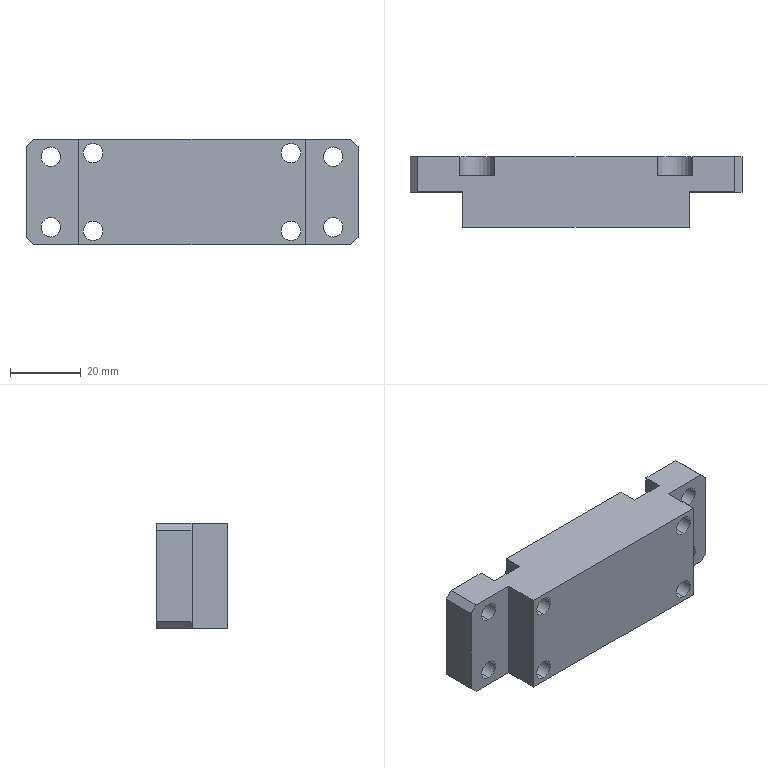Part | STEP file | 11-FG-SZ03311 | 1 solid | 48 faces | box 94 x 20 x 30 mm | volume 43270 mm3 | plane 26 | cylinder 22 | commonest cylinder face diameters 5.5 x16 10 x6
STEP:
#1=CARTESIAN_POINT('',(40.,10.,2.25));
#2=VERTEX_POINT('',#1);
#3=CARTESIAN_POINT('',(40.,10.,7.75));
#4=VERTEX_POINT('',#3);
#5=CARTESIAN_POINT('',(40.,10.,5.));
#6=DIRECTION('',(0.,1.,0.));
#7=DIRECTION('',(0.,0.,-1.));
#8=AXIS2_PLACEMENT_3D('',#5,#6,#7);
#9=CIRCLE('',#8,2.75);
#10=EDGE_CURVE('',#2,#4,#9,.T.);
#11=ORIENTED_EDGE('',*,*,#10,.T.);
#12=CARTESIAN_POINT('',(40.,0.,7.75));
#13=VERTEX_POINT('',#12);
#14=CARTESIAN_POINT('',(40.,18.,7.75));
#15=DIRECTION('',(0.,-1.,0.));
#16=VECTOR('',#15,1000.);
#17=LINE('',#14,#16);
#18=EDGE_CURVE('',#4,#13,#17,.T.);
#19=ORIENTED_EDGE('',*,*,#18,.T.);
#20=CARTESIAN_POINT('',(40.,0.,2.25));
#21=VERTEX_POINT('',#20);
#22=CARTESIAN_POINT('',(40.,0.,5.));
#23=DIRECTION('',(0.,1.,0.));
#24=DIRECTION('',(0.,0.,-1.));
#25=AXIS2_PLACEMENT_3D('',#22,#23,#24);
#26=CIRCLE('',#25,2.75);
#27=EDGE_CURVE('',#21,#13,#26,.T.);
#28=ORIENTED_EDGE('',*,*,#27,.F.);
#29=CARTESIAN_POINT('',(40.,18.,2.25));
#30=DIRECTION('',(0.,-1.,0.));
#31=VECTOR('',#30,1000.);
#32=LINE('',#29,#31);
#33=EDGE_CURVE('',#2,#21,#32,.T.);
#34=ORIENTED_EDGE('',*,*,#33,.F.);
#35=EDGE_LOOP('',(#11,#19,#28,#34));
#36=FACE_OUTER_BOUND('',#35,.T.);
#37=CARTESIAN_POINT('',(40.,18.,5.));
#38=DIRECTION('',(0.,-1.,0.));
#39=DIRECTION('',(0.,0.,-1.));
#40=AXIS2_PLACEMENT_3D('',#37,#38,#39);
#41=CYLINDRICAL_SURFACE('',#40,2.75);
#42=ADVANCED_FACE('',(#36),#41,.F.);
#43=CARTESIAN_POINT('',(40.,10.,22.25));
#44=VERTEX_POINT('',#43);
#45=CARTESIAN_POINT('',(40.,10.,27.75));
#46=VERTEX_POINT('',#45);
#47=CARTESIAN_POINT('',(40.,10.,25.));
#48=DIRECTION('',(0.,1.,0.));
#49=DIRECTION('',(0.,0.,-1.));
#50=AXIS2_PLACEMENT_3D('',#47,#48,#49);
#51=CIRCLE('',#50,2.75);
#52=EDGE_CURVE('',#44,#46,#51,.T.);
#53=ORIENTED_EDGE('',*,*,#52,.T.);
#54=CARTESIAN_POINT('',(40.,0.,27.75));
#55=VERTEX_POINT('',#54);
#56=CARTESIAN_POINT('',(40.,18.,27.75));
#57=DIRECTION('',(0.,-1.,0.));
#58=VECTOR('',#57,1000.);
#59=LINE('',#56,#58);
#60=EDGE_CURVE('',#46,#55,#59,.T.);
#61=ORIENTED_EDGE('',*,*,#60,.T.);
#62=CARTESIAN_POINT('',(40.,0.,22.25));
#63=VERTEX_POINT('',#62);
#64=CARTESIAN_POINT('',(40.,0.,25.));
#65=DIRECTION('',(0.,1.,0.));
#66=DIRECTION('',(0.,0.,-1.));
#67=AXIS2_PLACEMENT_3D('',#64,#65,#66);
#68=CIRCLE('',#67,2.75);
#69=EDGE_CURVE('',#63,#55,#68,.T.);
#70=ORIENTED_EDGE('',*,*,#69,.F.);
#71=CARTESIAN_POINT('',(40.,18.,22.25));
#72=DIRECTION('',(0.,-1.,0.));
#73=VECTOR('',#72,1000.);
#74=LINE('',#71,#73);
#75=EDGE_CURVE('',#44,#63,#74,.T.);
#76=ORIENTED_EDGE('',*,*,#75,.F.);
#77=EDGE_LOOP('',(#53,#61,#70,#76));
#78=FACE_OUTER_BOUND('',#77,.T.);
#79=CARTESIAN_POINT('',(40.,18.,25.));
#80=DIRECTION('',(0.,-1.,0.));
#81=DIRECTION('',(0.,0.,-1.));
#82=AXIS2_PLACEMENT_3D('',#79,#80,#81);
#83=CYLINDRICAL_SURFACE('',#82,2.75);
#84=ADVANCED_FACE('',(#78),#83,.F.);
#85=CARTESIAN_POINT('',(-40.,10.,7.75));
#86=VERTEX_POINT('',#85);
#87=CARTESIAN_POINT('',(-40.,10.,2.25));
#88=VERTEX_POINT('',#87);
#89=CARTESIAN_POINT('',(-40.,10.,5.));
#90=DIRECTION('',(0.,-1.,0.));
#91=DIRECTION('',(0.,0.,-1.));
#92=AXIS2_PLACEMENT_3D('',#89,#90,#91);
#93=CIRCLE('',#92,2.75);
#94=EDGE_CURVE('',#86,#88,#93,.T.);
#95=ORIENTED_EDGE('',*,*,#94,.F.);
#96=CARTESIAN_POINT('',(-40.,0.,7.75));
#97=VERTEX_POINT('',#96);
#98=CARTESIAN_POINT('',(-40.,18.,7.75));
#99=DIRECTION('',(0.,-1.,0.));
#100=VECTOR('',#99,1000.);
#101=LINE('',#98,#100);
#102=EDGE_CURVE('',#86,#97,#101,.T.);
#103=ORIENTED_EDGE('',*,*,#102,.T.);
#104=CARTESIAN_POINT('',(-40.,0.,2.25));
#105=VERTEX_POINT('',#104);
#106=CARTESIAN_POINT('',(-40.,0.,5.));
#107=DIRECTION('',(0.,-1.,0.));
#108=DIRECTION('',(0.,0.,-1.));
#109=AXIS2_PLACEMENT_3D('',#106,#107,#108);
#110=CIRCLE('',#109,2.75);
#111=EDGE_CURVE('',#97,#105,#110,.T.);
#112=ORIENTED_EDGE('',*,*,#111,.T.);
#113=CARTESIAN_POINT('',(-40.,18.,2.25));
#114=DIRECTION('',(0.,-1.,0.));
#115=VECTOR('',#114,1000.);
#116=LINE('',#113,#115);
#117=EDGE_CURVE('',#88,#105,#116,.T.);
#118=ORIENTED_EDGE('',*,*,#117,.F.);
#119=EDGE_LOOP('',(#95,#103,#112,#118));
#120=FACE_OUTER_BOUND('',#119,.T.);
#121=CARTESIAN_POINT('',(-40.,18.,5.));
#122=DIRECTION('',(0.,-1.,0.));
#123=DIRECTION('',(0.,0.,-1.));
#124=AXIS2_PLACEMENT_3D('',#121,#122,#123);
#125=CYLINDRICAL_SURFACE('',#124,2.75);
#126=ADVANCED_FACE('',(#120),#125,.F.);
#127=CARTESIAN_POINT('',(-40.,10.,27.75));
#128=VERTEX_POINT('',#127);
#129=CARTESIAN_POINT('',(-40.,10.,22.25));
#130=VERTEX_POINT('',#129);
#131=CARTESIAN_POINT('',(-40.,10.,25.));
#132=DIRECTION('',(0.,-1.,0.));
#133=DIRECTION('',(0.,0.,-1.));
#134=AXIS2_PLACEMENT_3D('',#131,#132,#133);
#135=CIRCLE('',#134,2.75);
#136=EDGE_CURVE('',#128,#130,#135,.T.);
#137=ORIENTED_EDGE('',*,*,#136,.F.);
#138=CARTESIAN_POINT('',(-40.,0.,27.75));
#139=VERTEX_POINT('',#138);
#140=CARTESIAN_POINT('',(-40.,18.,27.75));
#141=DIRECTION('',(0.,-1.,0.));
#142=VECTOR('',#141,1000.);
#143=LINE('',#140,#142);
#144=EDGE_CURVE('',#128,#139,#143,.T.);
#145=ORIENTED_EDGE('',*,*,#144,.T.);
#146=CARTESIAN_POINT('',(-40.,0.,22.25));
#147=VERTEX_POINT('',#146);
#148=CARTESIAN_POINT('',(-40.,0.,25.));
#149=DIRECTION('',(0.,-1.,0.));
#150=DIRECTION('',(0.,0.,-1.));
#151=AXIS2_PLACEMENT_3D('',#148,#149,#150);
#152=CIRCLE('',#151,2.75);
#153=EDGE_CURVE('',#139,#147,#152,.T.);
#154=ORIENTED_EDGE('',*,*,#153,.T.);
#155=CARTESIAN_POINT('',(-40.,18.,22.25));
#156=DIRECTION('',(0.,-1.,0.));
#157=VECTOR('',#156,1000.);
#158=LINE('',#155,#157);
#159=EDGE_CURVE('',#130,#147,#158,.T.);
#160=ORIENTED_EDGE('',*,*,#159,.F.);
#161=EDGE_LOOP('',(#137,#145,#154,#160));
#162=FACE_OUTER_BOUND('',#161,.T.);
#163=CARTESIAN_POINT('',(-40.,18.,25.));
#164=DIRECTION('',(0.,-1.,0.));
#165=DIRECTION('',(0.,0.,-1.));
#166=AXIS2_PLACEMENT_3D('',#163,#164,#165);
#167=CYLINDRICAL_SURFACE('',#166,2.75);
#168=ADVANCED_FACE('',(#162),#167,.F.);
#169=CARTESIAN_POINT('',(28.,-10.,23.25));
#170=VERTEX_POINT('',#169);
#171=CARTESIAN_POINT('',(28.,-10.,28.75));
#172=VERTEX_POINT('',#171);
#173=CARTESIAN_POINT('',(28.,-10.,26.));
#174=DIRECTION('',(0.,1.,0.));
#175=DIRECTION('',(0.,0.,1.));
#176=AXIS2_PLACEMENT_3D('',#173,#174,#175);
#177=CIRCLE('',#176,2.75);
#178=EDGE_CURVE('',#170,#172,#177,.T.);
#179=ORIENTED_EDGE('',*,*,#178,.F.);
#180=CARTESIAN_POINT('',(28.,4.6,23.25));
#181=VERTEX_POINT('',#180);
#182=CARTESIAN_POINT('',(28.,10.,23.25));
#183=DIRECTION('',(0.,1.,0.));
#184=VECTOR('',#183,1000.);
#185=LINE('',#182,#184);
#186=EDGE_CURVE('',#170,#181,#185,.T.);
#187=ORIENTED_EDGE('',*,*,#186,.T.);
#188=CARTESIAN_POINT('',(28.,4.6,28.75));
#189=VERTEX_POINT('',#188);
#190=CARTESIAN_POINT('',(28.,4.6,26.));
#191=DIRECTION('',(0.,1.,0.));
#192=DIRECTION('',(0.,0.,1.));
#193=AXIS2_PLACEMENT_3D('',#190,#191,#192);
#194=CIRCLE('',#193,2.75);
#195=EDGE_CURVE('',#181,#189,#194,.T.);
#196=ORIENTED_EDGE('',*,*,#195,.T.);
#197=CARTESIAN_POINT('',(28.,10.,28.75));
#198=DIRECTION('',(0.,1.,0.));
#199=VECTOR('',#198,1000.);
#200=LINE('',#197,#199);
#201=EDGE_CURVE('',#172,#189,#200,.T.);
#202=ORIENTED_EDGE('',*,*,#201,.F.);
#203=EDGE_LOOP('',(#179,#187,#196,#202));
#204=FACE_OUTER_BOUND('',#203,.T.);
#205=CARTESIAN_POINT('',(28.,10.,26.));
#206=DIRECTION('',(0.,1.,0.));
#207=DIRECTION('',(0.,0.,1.));
#208=AXIS2_PLACEMENT_3D('',#205,#206,#207);
#209=CYLINDRICAL_SURFACE('',#208,2.75);
#210=ADVANCED_FACE('',(#204),#209,.F.);
#211=CARTESIAN_POINT('',(28.,4.6,9.));
#212=VERTEX_POINT('',#211);
#213=CARTESIAN_POINT('',(33.,4.6,4.));
#214=VERTEX_POINT('',#213);
#215=CARTESIAN_POINT('',(28.,4.6,4.));
#216=DIRECTION('',(0.,1.,0.));
#217=DIRECTION('',(0.,0.,1.));
#218=AXIS2_PLACEMENT_3D('',#215,#216,#217);
#219=CIRCLE('',#218,5.);
#220=EDGE_CURVE('',#212,#214,#219,.T.);
#221=ORIENTED_EDGE('',*,*,#220,.F.);
#222=CARTESIAN_POINT('',(28.,10.,9.));
#223=VERTEX_POINT('',#222);
#224=CARTESIAN_POINT('',(28.,10.,9.));
#225=DIRECTION('',(0.,1.,0.));
#226=VECTOR('',#225,1000.);
#227=LINE('',#224,#226);
#228=EDGE_CURVE('',#212,#223,#227,.T.);
#229=ORIENTED_EDGE('',*,*,#228,.T.);
#230=CARTESIAN_POINT('',(33.,10.,4.));
#231=VERTEX_POINT('',#230);
#232=CARTESIAN_POINT('',(28.,10.,4.));
#233=DIRECTION('',(0.,1.,0.));
#234=DIRECTION('',(0.,0.,1.));
#235=AXIS2_PLACEMENT_3D('',#232,#233,#234);
#236=CIRCLE('',#235,5.);
#237=EDGE_CURVE('',#223,#231,#236,.T.);
#238=ORIENTED_EDGE('',*,*,#237,.T.);
#239=CARTESIAN_POINT('',(33.,-6.17,4.));
#240=DIRECTION('',(0.,1.,0.));
#241=VECTOR('',#240,1000.);
#242=LINE('',#239,#241);
#243=EDGE_CURVE('',#214,#231,#242,.T.);
#244=ORIENTED_EDGE('',*,*,#243,.F.);
#245=EDGE_LOOP('',(#221,#229,#238,#244));
#246=FACE_OUTER_BOUND('',#245,.T.);
#247=CARTESIAN_POINT('',(28.,10.,4.));
#248=DIRECTION('',(0.,1.,0.));
#249=DIRECTION('',(0.,0.,1.));
#250=AXIS2_PLACEMENT_3D('',#247,#248,#249);
#251=CYLINDRICAL_SURFACE('',#250,5.);
#252=ADVANCED_FACE('',(#246),#251,.F.);
#253=CARTESIAN_POINT('',(28.,-10.,1.25));
#254=VERTEX_POINT('',#253);
#255=CARTESIAN_POINT('',(28.,-10.,6.75));
#256=VERTEX_POINT('',#255);
#257=CARTESIAN_POINT('',(28.,-10.,4.));
#258=DIRECTION('',(0.,1.,0.));
#259=DIRECTION('',(0.,0.,1.));
#260=AXIS2_PLACEMENT_3D('',#257,#258,#259);
#261=CIRCLE('',#260,2.75);
#262=EDGE_CURVE('',#254,#256,#261,.T.);
#263=ORIENTED_EDGE('',*,*,#262,.F.);
#264=CARTESIAN_POINT('',(28.,4.6,1.25));
#265=VERTEX_POINT('',#264);
#266=CARTESIAN_POINT('',(28.,10.,1.25));
#267=DIRECTION('',(0.,1.,0.));
#268=VECTOR('',#267,1000.);
#269=LINE('',#266,#268);
#270=EDGE_CURVE('',#254,#265,#269,.T.);
#271=ORIENTED_EDGE('',*,*,#270,.T.);
#272=CARTESIAN_POINT('',(28.,4.6,6.75));
#273=VERTEX_POINT('',#272);
#274=CARTESIAN_POINT('',(28.,4.6,4.));
#275=DIRECTION('',(0.,1.,0.));
#276=DIRECTION('',(0.,0.,1.));
#277=AXIS2_PLACEMENT_3D('',#274,#275,#276);
#278=CIRCLE('',#277,2.75);
#279=EDGE_CURVE('',#265,#273,#278,.T.);
#280=ORIENTED_EDGE('',*,*,#279,.T.);
#281=CARTESIAN_POINT('',(28.,10.,6.75));
#282=DIRECTION('',(0.,1.,0.));
#283=VECTOR('',#282,1000.);
#284=LINE('',#281,#283);
#285=EDGE_CURVE('',#256,#273,#284,.T.);
#286=ORIENTED_EDGE('',*,*,#285,.F.);
#287=EDGE_LOOP('',(#263,#271,#280,#286));
#288=FACE_OUTER_BOUND('',#287,.T.);
#289=CARTESIAN_POINT('',(28.,10.,4.));
#290=DIRECTION('',(0.,1.,0.));
#291=DIRECTION('',(0.,0.,1.));
#292=AXIS2_PLACEMENT_3D('',#289,#290,#291);
#293=CYLINDRICAL_SURFACE('',#292,2.75);
#294=ADVANCED_FACE('',(#288),#293,.F.);
#295=CARTESIAN_POINT('',(-28.,-10.,23.25));
#296=VERTEX_POINT('',#295);
#297=CARTESIAN_POINT('',(-28.,-10.,28.75));
#298=VERTEX_POINT('',#297);
#299=CARTESIAN_POINT('',(-28.,-10.,26.));
#300=DIRECTION('',(0.,1.,0.));
#301=DIRECTION('',(0.,0.,1.));
#302=AXIS2_PLACEMENT_3D('',#299,#300,#301);
#303=CIRCLE('',#302,2.75);
#304=EDGE_CURVE('',#296,#298,#303,.T.);
#305=ORIENTED_EDGE('',*,*,#304,.F.);
#306=CARTESIAN_POINT('',(-28.,4.6,23.25));
#307=VERTEX_POINT('',#306);
#308=CARTESIAN_POINT('',(-28.,10.,23.25));
#309=DIRECTION('',(0.,1.,0.));
#310=VECTOR('',#309,1000.);
#311=LINE('',#308,#310);
#312=EDGE_CURVE('',#296,#307,#311,.T.);
#313=ORIENTED_EDGE('',*,*,#312,.T.);
#314=CARTESIAN_POINT('',(-28.,4.6,28.75));
#315=VERTEX_POINT('',#314);
#316=CARTESIAN_POINT('',(-28.,4.6,26.));
#317=DIRECTION('',(0.,1.,0.));
#318=DIRECTION('',(0.,0.,1.));
#319=AXIS2_PLACEMENT_3D('',#316,#317,#318);
#320=CIRCLE('',#319,2.75);
#321=EDGE_CURVE('',#307,#315,#320,.T.);
#322=ORIENTED_EDGE('',*,*,#321,.T.);
#323=CARTESIAN_POINT('',(-28.,10.,28.75));
#324=DIRECTION('',(0.,1.,0.));
#325=VECTOR('',#324,1000.);
#326=LINE('',#323,#325);
#327=EDGE_CURVE('',#298,#315,#326,.T.);
#328=ORIENTED_EDGE('',*,*,#327,.F.);
#329=EDGE_LOOP('',(#305,#313,#322,#328));
#330=FACE_OUTER_BOUND('',#329,.T.);
#331=CARTESIAN_POINT('',(-28.,10.,26.));
#332=DIRECTION('',(0.,1.,0.));
#333=DIRECTION('',(0.,0.,1.));
#334=AXIS2_PLACEMENT_3D('',#331,#332,#333);
#335=CYLINDRICAL_SURFACE('',#334,2.75);
#336=ADVANCED_FACE('',(#330),#335,.F.);
#337=CARTESIAN_POINT('',(-28.,4.6,9.));
#338=VERTEX_POINT('',#337);
#339=CARTESIAN_POINT('',(-23.,4.6,4.));
#340=VERTEX_POINT('',#339);
#341=CARTESIAN_POINT('',(-28.,4.6,4.));
#342=DIRECTION('',(0.,1.,0.));
#343=DIRECTION('',(0.,0.,1.));
#344=AXIS2_PLACEMENT_3D('',#341,#342,#343);
#345=CIRCLE('',#344,5.);
#346=EDGE_CURVE('',#338,#340,#345,.T.);
#347=ORIENTED_EDGE('',*,*,#346,.F.);
#348=CARTESIAN_POINT('',(-28.,10.,9.));
#349=VERTEX_POINT('',#348);
#350=CARTESIAN_POINT('',(-28.,10.,9.));
#351=DIRECTION('',(0.,1.,0.));
#352=VECTOR('',#351,1000.);
#353=LINE('',#350,#352);
#354=EDGE_CURVE('',#338,#349,#353,.T.);
#355=ORIENTED_EDGE('',*,*,#354,.T.);
#356=CARTESIAN_POINT('',(-23.,10.,4.));
#357=VERTEX_POINT('',#356);
#358=CARTESIAN_POINT('',(-28.,10.,4.));
#359=DIRECTION('',(0.,1.,0.));
#360=DIRECTION('',(0.,0.,1.));
#361=AXIS2_PLACEMENT_3D('',#358,#359,#360);
#362=CIRCLE('',#361,5.);
#363=EDGE_CURVE('',#349,#357,#362,.T.);
#364=ORIENTED_EDGE('',*,*,#363,.T.);
#365=CARTESIAN_POINT('',(-23.,-6.17,4.));
#366=DIRECTION('',(0.,1.,0.));
#367=VECTOR('',#366,1000.);
#368=LINE('',#365,#367);
#369=EDGE_CURVE('',#340,#357,#368,.T.);
#370=ORIENTED_EDGE('',*,*,#369,.F.);
#371=EDGE_LOOP('',(#347,#355,#364,#370));
#372=FACE_OUTER_BOUND('',#371,.T.);
#373=CARTESIAN_POINT('',(-28.,10.,4.));
#374=DIRECTION('',(0.,1.,0.));
#375=DIRECTION('',(0.,0.,1.));
#376=AXIS2_PLACEMENT_3D('',#373,#374,#375);
#377=CYLINDRICAL_SURFACE('',#376,5.);
#378=ADVANCED_FACE('',(#372),#377,.F.);
#379=CARTESIAN_POINT('',(-28.,-10.,1.25));
#380=VERTEX_POINT('',#379);
#381=CARTESIAN_POINT('',(-28.,-10.,6.75));
#382=VERTEX_POINT('',#381);
#383=CARTESIAN_POINT('',(-28.,-10.,4.));
#384=DIRECTION('',(0.,1.,0.));
#385=DIRECTION('',(0.,0.,1.));
#386=AXIS2_PLACEMENT_3D('',#383,#384,#385);
#387=CIRCLE('',#386,2.75);
#388=EDGE_CURVE('',#380,#382,#387,.T.);
#389=ORIENTED_EDGE('',*,*,#388,.F.);
#390=CARTESIAN_POINT('',(-28.,4.6,1.25));
#391=VERTEX_POINT('',#390);
#392=CARTESIAN_POINT('',(-28.,10.,1.25));
#393=DIRECTION('',(0.,1.,0.));
#394=VECTOR('',#393,1000.);
#395=LINE('',#392,#394);
#396=EDGE_CURVE('',#380,#391,#395,.T.);
#397=ORIENTED_EDGE('',*,*,#396,.T.);
#398=CARTESIAN_POINT('',(-28.,4.6,6.75));
#399=VERTEX_POINT('',#398);
#400=CARTESIAN_POINT('',(-28.,4.6,4.));
#401=DIRECTION('',(0.,1.,0.));
#402=DIRECTION('',(0.,0.,1.));
#403=AXIS2_PLACEMENT_3D('',#400,#401,#402);
#404=CIRCLE('',#403,2.75);
#405=EDGE_CURVE('',#391,#399,#404,.T.);
#406=ORIENTED_EDGE('',*,*,#405,.T.);
#407=CARTESIAN_POINT('',(-28.,10.,6.75));
#408=DIRECTION('',(0.,1.,0.));
#409=VECTOR('',#408,1000.);
#410=LINE('',#407,#409);
#411=EDGE_CURVE('',#382,#399,#410,.T.);
#412=ORIENTED_EDGE('',*,*,#411,.F.);
#413=EDGE_LOOP('',(#389,#397,#406,#412));
#414=FACE_OUTER_BOUND('',#413,.T.);
#415=CARTESIAN_POINT('',(-28.,10.,4.));
#416=DIRECTION('',(0.,1.,0.));
#417=DIRECTION('',(0.,0.,1.));
#418=AXIS2_PLACEMENT_3D('',#415,#416,#417);
#419=CYLINDRICAL_SURFACE('',#418,2.75);
#420=ADVANCED_FACE('',(#414),#419,.F.);
#421=CARTESIAN_POINT('',(-23.,10.,26.));
#422=VERTEX_POINT('',#421);
#423=CARTESIAN_POINT('',(-33.,10.,26.));
#424=VERTEX_POINT('',#423);
#425=CARTESIAN_POINT('',(-28.,10.,26.));
#426=DIRECTION('',(0.,1.,0.));
#427=DIRECTION('',(0.,0.,1.));
#428=AXIS2_PLACEMENT_3D('',#425,#426,#427);
#429=CIRCLE('',#428,5.);
#430=EDGE_CURVE('',#422,#424,#429,.T.);
#431=ORIENTED_EDGE('',*,*,#430,.T.);
#432=CARTESIAN_POINT('',(-33.,4.6,26.));
#433=VERTEX_POINT('',#432);
#434=CARTESIAN_POINT('',(-33.,-6.17,26.));
#435=DIRECTION('',(0.,1.,0.));
#436=VECTOR('',#435,1000.);
#437=LINE('',#434,#436);
#438=EDGE_CURVE('',#433,#424,#437,.T.);
#439=ORIENTED_EDGE('',*,*,#438,.F.);
#440=CARTESIAN_POINT('',(-23.,4.6,26.));
#441=VERTEX_POINT('',#440);
#442=CARTESIAN_POINT('',(-28.,4.6,26.));
#443=DIRECTION('',(0.,1.,0.));
#444=DIRECTION('',(0.,0.,1.));
#445=AXIS2_PLACEMENT_3D('',#442,#443,#444);
#446=CIRCLE('',#445,5.);
#447=EDGE_CURVE('',#441,#433,#446,.T.);
#448=ORIENTED_EDGE('',*,*,#447,.F.);
#449=CARTESIAN_POINT('',(-23.,-6.17,26.));
#450=DIRECTION('',(0.,1.,0.));
#451=VECTOR('',#450,1000.);
#452=LINE('',#449,#451);
#453=EDGE_CURVE('',#441,#422,#452,.T.);
#454=ORIENTED_EDGE('',*,*,#453,.T.);
#455=EDGE_LOOP('',(#431,#439,#448,#454));
#456=FACE_OUTER_BOUND('',#455,.T.);
#457=CARTESIAN_POINT('',(-28.,10.,26.));
#458=DIRECTION('',(0.,1.,0.));
#459=DIRECTION('',(0.,0.,1.));
#460=AXIS2_PLACEMENT_3D('',#457,#458,#459);
#461=CYLINDRICAL_SURFACE('',#460,5.);
#462=ADVANCED_FACE('',(#456),#461,.F.);
#463=CARTESIAN_POINT('',(33.,10.,26.));
#464=VERTEX_POINT('',#463);
#465=CARTESIAN_POINT('',(23.,10.,26.));
#466=VERTEX_POINT('',#465);
#467=CARTESIAN_POINT('',(28.,10.,26.));
#468=DIRECTION('',(0.,1.,0.));
#469=DIRECTION('',(0.,0.,1.));
#470=AXIS2_PLACEMENT_3D('',#467,#468,#469);
#471=CIRCLE('',#470,5.);
#472=EDGE_CURVE('',#464,#466,#471,.T.);
#473=ORIENTED_EDGE('',*,*,#472,.T.);
#474=CARTESIAN_POINT('',(23.,4.6,26.));
#475=VERTEX_POINT('',#474);
#476=CARTESIAN_POINT('',(23.,-6.17,26.));
#477=DIRECTION('',(0.,1.,0.));
#478=VECTOR('',#477,1000.);
#479=LINE('',#476,#478);
#480=EDGE_CURVE('',#475,#466,#479,.T.);
#481=ORIENTED_EDGE('',*,*,#480,.F.);
#482=CARTESIAN_POINT('',(33.,4.6,26.));
#483=VERTEX_POINT('',#482);
#484=CARTESIAN_POINT('',(28.,4.6,26.));
#485=DIRECTION('',(0.,1.,0.));
#486=DIRECTION('',(0.,0.,1.));
#487=AXIS2_PLACEMENT_3D('',#484,#485,#486);
#488=CIRCLE('',#487,5.);
#489=EDGE_CURVE('',#483,#475,#488,.T.);
#490=ORIENTED_EDGE('',*,*,#489,.F.);
#491=CARTESIAN_POINT('',(33.,-6.17,26.));
#492=DIRECTION('',(0.,1.,0.));
#493=VECTOR('',#492,1000.);
#494=LINE('',#491,#493);
#495=EDGE_CURVE('',#483,#464,#494,.T.);
#496=ORIENTED_EDGE('',*,*,#495,.T.);
#497=EDGE_LOOP('',(#473,#481,#490,#496));
#498=FACE_OUTER_BOUND('',#497,.T.);
#499=CARTESIAN_POINT('',(28.,10.,26.));
#500=DIRECTION('',(0.,1.,0.));
#501=DIRECTION('',(0.,0.,1.));
#502=AXIS2_PLACEMENT_3D('',#499,#500,#501);
#503=CYLINDRICAL_SURFACE('',#502,5.);
#504=ADVANCED_FACE('',(#498),#503,.F.);
#505=ORIENTED_EDGE('',*,*,#10,.F.);
#506=CARTESIAN_POINT('',(40.,10.,5.));
#507=DIRECTION('',(0.,1.,0.));
#508=DIRECTION('',(0.,0.,-1.));
#509=AXIS2_PLACEMENT_3D('',#506,#507,#508);
#510=CIRCLE('',#509,2.75);
#511=EDGE_CURVE('',#4,#2,#510,.T.);
#512=ORIENTED_EDGE('',*,*,#511,.F.);
#513=EDGE_LOOP('',(#505,#512));
#514=FACE_BOUND('',#513,.T.);
#515=ORIENTED_EDGE('',*,*,#52,.F.);
#516=CARTESIAN_POINT('',(40.,10.,25.));
#517=DIRECTION('',(0.,1.,0.));
#518=DIRECTION('',(0.,0.,-1.));
#519=AXIS2_PLACEMENT_3D('',#516,#517,#518);
#520=CIRCLE('',#519,2.75);
#521=EDGE_CURVE('',#46,#44,#520,.T.);
#522=ORIENTED_EDGE('',*,*,#521,.F.);
#523=EDGE_LOOP('',(#515,#522));
#524=FACE_BOUND('',#523,.T.);
#525=CARTESIAN_POINT('',(-40.,10.,5.));
#526=DIRECTION('',(0.,-1.,0.));
#527=DIRECTION('',(0.,0.,-1.));
#528=AXIS2_PLACEMENT_3D('',#525,#526,#527);
#529=CIRCLE('',#528,2.75);
#530=EDGE_CURVE('',#88,#86,#529,.T.);
#531=ORIENTED_EDGE('',*,*,#530,.T.);
#532=ORIENTED_EDGE('',*,*,#94,.T.);
#533=EDGE_LOOP('',(#531,#532));
#534=FACE_BOUND('',#533,.T.);
#535=CARTESIAN_POINT('',(-40.,10.,25.));
#536=DIRECTION('',(0.,-1.,0.));
#537=DIRECTION('',(0.,0.,-1.));
#538=AXIS2_PLACEMENT_3D('',#535,#536,#537);
#539=CIRCLE('',#538,2.75);
#540=EDGE_CURVE('',#130,#128,#539,.T.);
#541=ORIENTED_EDGE('',*,*,#540,.T.);
#542=ORIENTED_EDGE('',*,*,#136,.T.);
#543=EDGE_LOOP('',(#541,#542));
#544=FACE_BOUND('',#543,.T.);
#545=CARTESIAN_POINT('',(-33.,10.,0.));
#546=VERTEX_POINT('',#545);
#547=CARTESIAN_POINT('',(-45.,10.,0.));
#548=VERTEX_POINT('',#547);
#549=CARTESIAN_POINT('',(-47.,10.,0.));
#550=DIRECTION('',(-1.,0.,0.));
#551=VECTOR('',#550,1000.);
#552=LINE('',#549,#551);
#553=EDGE_CURVE('',#546,#548,#552,.T.);
#554=ORIENTED_EDGE('',*,*,#553,.T.);
#555=CARTESIAN_POINT('',(-47.,10.,2.));
#556=VERTEX_POINT('',#555);
#557=CARTESIAN_POINT('',(-47.,10.,2.));
#558=DIRECTION('',(-0.7071,0.,0.7071));
#559=VECTOR('',#558,1000.);
#560=LINE('',#557,#559);
#561=EDGE_CURVE('',#548,#556,#560,.T.);
#562=ORIENTED_EDGE('',*,*,#561,.T.);
#563=CARTESIAN_POINT('',(-47.,10.,28.));
#564=VERTEX_POINT('',#563);
#565=CARTESIAN_POINT('',(-47.,10.,30.));
#566=DIRECTION('',(0.,0.,-1.));
#567=VECTOR('',#566,1000.);
#568=LINE('',#565,#567);
#569=EDGE_CURVE('',#564,#556,#568,.T.);
#570=ORIENTED_EDGE('',*,*,#569,.F.);
#571=CARTESIAN_POINT('',(-45.,10.,30.));
#572=VERTEX_POINT('',#571);
#573=CARTESIAN_POINT('',(-45.,10.,30.));
#574=DIRECTION('',(0.7071,0.,0.7071));
#575=VECTOR('',#574,1000.);
#576=LINE('',#573,#575);
#577=EDGE_CURVE('',#564,#572,#576,.T.);
#578=ORIENTED_EDGE('',*,*,#577,.T.);
#579=CARTESIAN_POINT('',(-33.,10.,30.));
#580=VERTEX_POINT('',#579);
#581=CARTESIAN_POINT('',(-47.,10.,30.));
#582=DIRECTION('',(-1.,0.,0.));
#583=VECTOR('',#582,1000.);
#584=LINE('',#581,#583);
#585=EDGE_CURVE('',#580,#572,#584,.T.);
#586=ORIENTED_EDGE('',*,*,#585,.F.);
#587=CARTESIAN_POINT('',(-33.,10.,26.));
#588=DIRECTION('',(0.,0.,1.));
#589=VECTOR('',#588,1000.);
#590=LINE('',#587,#589);
#591=EDGE_CURVE('',#424,#580,#590,.T.);
#592=ORIENTED_EDGE('',*,*,#591,.F.);
#593=ORIENTED_EDGE('',*,*,#430,.F.);
#594=CARTESIAN_POINT('',(-23.,10.,30.));
#595=VERTEX_POINT('',#594);
#596=CARTESIAN_POINT('',(-23.,10.,26.));
#597=DIRECTION('',(0.,0.,-1.));
#598=VECTOR('',#597,1000.);
#599=LINE('',#596,#598);
#600=EDGE_CURVE('',#595,#422,#599,.T.);
#601=ORIENTED_EDGE('',*,*,#600,.F.);
#602=CARTESIAN_POINT('',(23.,10.,30.));
#603=VERTEX_POINT('',#602);
#604=CARTESIAN_POINT('',(-47.,10.,30.));
#605=DIRECTION('',(-1.,0.,0.));
#606=VECTOR('',#605,1000.);
#607=LINE('',#604,#606);
#608=EDGE_CURVE('',#603,#595,#607,.T.);
#609=ORIENTED_EDGE('',*,*,#608,.F.);
#610=CARTESIAN_POINT('',(23.,10.,26.));
#611=DIRECTION('',(0.,0.,1.));
#612=VECTOR('',#611,1000.);
#613=LINE('',#610,#612);
#614=EDGE_CURVE('',#466,#603,#613,.T.);
#615=ORIENTED_EDGE('',*,*,#614,.F.);
#616=ORIENTED_EDGE('',*,*,#472,.F.);
#617=CARTESIAN_POINT('',(33.,10.,30.));
#618=VERTEX_POINT('',#617);
#619=CARTESIAN_POINT('',(33.,10.,26.));
#620=DIRECTION('',(0.,0.,-1.));
#621=VECTOR('',#620,1000.);
#622=LINE('',#619,#621);
#623=EDGE_CURVE('',#618,#464,#622,.T.);
#624=ORIENTED_EDGE('',*,*,#623,.F.);
#625=CARTESIAN_POINT('',(45.,10.,30.));
#626=VERTEX_POINT('',#625);
#627=CARTESIAN_POINT('',(-47.,10.,30.));
#628=DIRECTION('',(-1.,0.,0.));
#629=VECTOR('',#628,1000.);
#630=LINE('',#627,#629);
#631=EDGE_CURVE('',#626,#618,#630,.T.);
#632=ORIENTED_EDGE('',*,*,#631,.F.);
#633=CARTESIAN_POINT('',(47.,10.,28.));
#634=VERTEX_POINT('',#633);
#635=CARTESIAN_POINT('',(45.,10.,30.));
#636=DIRECTION('',(0.7071,0.,-0.7071));
#637=VECTOR('',#636,1000.);
#638=LINE('',#635,#637);
#639=EDGE_CURVE('',#626,#634,#638,.T.);
#640=ORIENTED_EDGE('',*,*,#639,.T.);
#641=CARTESIAN_POINT('',(47.,10.,2.));
#642=VERTEX_POINT('',#641);
#643=CARTESIAN_POINT('',(47.,10.,30.));
#644=DIRECTION('',(0.,0.,-1.));
#645=VECTOR('',#644,1000.);
#646=LINE('',#643,#645);
#647=EDGE_CURVE('',#634,#642,#646,.T.);
#648=ORIENTED_EDGE('',*,*,#647,.T.);
#649=CARTESIAN_POINT('',(45.,10.,0.));
#650=VERTEX_POINT('',#649);
#651=CARTESIAN_POINT('',(47.,10.,2.));
#652=DIRECTION('',(-0.7071,0.,-0.7071));
#653=VECTOR('',#652,1000.);
#654=LINE('',#651,#653);
#655=EDGE_CURVE('',#642,#650,#654,.T.);
#656=ORIENTED_EDGE('',*,*,#655,.T.);
#657=CARTESIAN_POINT('',(33.,10.,0.));
#658=VERTEX_POINT('',#657);
#659=CARTESIAN_POINT('',(-47.,10.,0.));
#660=DIRECTION('',(-1.,0.,0.));
#661=VECTOR('',#660,1000.);
#662=LINE('',#659,#661);
#663=EDGE_CURVE('',#650,#658,#662,.T.);
#664=ORIENTED_EDGE('',*,*,#663,.T.);
#665=CARTESIAN_POINT('',(33.,10.,4.));
#666=DIRECTION('',(0.,0.,-1.));
#667=VECTOR('',#666,1000.);
#668=LINE('',#665,#667);
#669=EDGE_CURVE('',#231,#658,#668,.T.);
#670=ORIENTED_EDGE('',*,*,#669,.F.);
#671=ORIENTED_EDGE('',*,*,#237,.F.);
#672=CARTESIAN_POINT('',(23.,10.,4.));
#673=VERTEX_POINT('',#672);
#674=CARTESIAN_POINT('',(28.,10.,4.));
#675=DIRECTION('',(0.,1.,0.));
#676=DIRECTION('',(0.,0.,1.));
#677=AXIS2_PLACEMENT_3D('',#674,#675,#676);
#678=CIRCLE('',#677,5.);
#679=EDGE_CURVE('',#673,#223,#678,.T.);
#680=ORIENTED_EDGE('',*,*,#679,.F.);
#681=CARTESIAN_POINT('',(23.,10.,0.));
#682=VERTEX_POINT('',#681);
#683=CARTESIAN_POINT('',(23.,10.,4.));
#684=DIRECTION('',(0.,0.,1.));
#685=VECTOR('',#684,1000.);
#686=LINE('',#683,#685);
#687=EDGE_CURVE('',#682,#673,#686,.T.);
#688=ORIENTED_EDGE('',*,*,#687,.F.);
#689=CARTESIAN_POINT('',(-23.,10.,0.));
#690=VERTEX_POINT('',#689);
#691=CARTESIAN_POINT('',(-47.,10.,0.));
#692=DIRECTION('',(-1.,0.,0.));
#693=VECTOR('',#692,1000.);
#694=LINE('',#691,#693);
#695=EDGE_CURVE('',#682,#690,#694,.T.);
#696=ORIENTED_EDGE('',*,*,#695,.T.);
#697=CARTESIAN_POINT('',(-23.,10.,4.));
#698=DIRECTION('',(0.,0.,-1.));
#699=VECTOR('',#698,1000.);
#700=LINE('',#697,#699);
#701=EDGE_CURVE('',#357,#690,#700,.T.);
#702=ORIENTED_EDGE('',*,*,#701,.F.);
#703=ORIENTED_EDGE('',*,*,#363,.F.);
#704=CARTESIAN_POINT('',(-33.,10.,4.));
#705=VERTEX_POINT('',#704);
#706=CARTESIAN_POINT('',(-28.,10.,4.));
#707=DIRECTION('',(0.,1.,0.));
#708=DIRECTION('',(0.,0.,1.));
#709=AXIS2_PLACEMENT_3D('',#706,#707,#708);
#710=CIRCLE('',#709,5.);
#711=EDGE_CURVE('',#705,#349,#710,.T.);
#712=ORIENTED_EDGE('',*,*,#711,.F.);
#713=CARTESIAN_POINT('',(-33.,10.,4.));
#714=DIRECTION('',(0.,0.,1.));
#715=VECTOR('',#714,1000.);
#716=LINE('',#713,#715);
#717=EDGE_CURVE('',#546,#705,#716,.T.);
#718=ORIENTED_EDGE('',*,*,#717,.F.);
#719=EDGE_LOOP('',(#554,#562,#570,#578,#586,#592,#593,#601,#609,#615,#616,#624,#632,#640,#648,#656,#664,#670,#671,#680,#688,#696,#702,#703,#712,#718));
#720=FACE_OUTER_BOUND('',#719,.T.);
#721=CARTESIAN_POINT('',(-47.,10.,30.));
#722=DIRECTION('',(0.,-1.,0.));
#723=DIRECTION('',(0.,0.,-1.));
#724=AXIS2_PLACEMENT_3D('',#721,#722,#723);
#725=PLANE('',#724);
#726=ADVANCED_FACE('',(#514,#524,#534,#544,#720),#725,.F.);
#727=ORIENTED_EDGE('',*,*,#647,.F.);
#728=CARTESIAN_POINT('',(47.,0.,28.));
#729=VERTEX_POINT('',#728);
#730=CARTESIAN_POINT('',(47.,-10.,28.));
#731=DIRECTION('',(0.,-1.,0.));
#732=VECTOR('',#731,1000.);
#733=LINE('',#730,#732);
#734=EDGE_CURVE('',#634,#729,#733,.T.);
#735=ORIENTED_EDGE('',*,*,#734,.T.);
#736=CARTESIAN_POINT('',(47.,0.,2.));
#737=VERTEX_POINT('',#736);
#738=CARTESIAN_POINT('',(47.,0.,0.));
#739=DIRECTION('',(0.,0.,1.));
#740=VECTOR('',#739,1000.);
#741=LINE('',#738,#740);
#742=EDGE_CURVE('',#737,#729,#741,.T.);
#743=ORIENTED_EDGE('',*,*,#742,.F.);
#744=CARTESIAN_POINT('',(47.,10.,2.));
#745=DIRECTION('',(0.,1.,0.));
#746=VECTOR('',#745,1000.);
#747=LINE('',#744,#746);
#748=EDGE_CURVE('',#737,#642,#747,.T.);
#749=ORIENTED_EDGE('',*,*,#748,.T.);
#750=EDGE_LOOP('',(#727,#735,#743,#749));
#751=FACE_OUTER_BOUND('',#750,.T.);
#752=CARTESIAN_POINT('',(47.,-10.,30.));
#753=DIRECTION('',(-1.,0.,0.));
#754=DIRECTION('',(0.,0.,1.));
#755=AXIS2_PLACEMENT_3D('',#752,#753,#754);
#756=PLANE('',#755);
#757=ADVANCED_FACE('',(#751),#756,.F.);
#758=ORIENTED_EDGE('',*,*,#569,.T.);
#759=CARTESIAN_POINT('',(-47.,0.,2.));
#760=VERTEX_POINT('',#759);
#761=CARTESIAN_POINT('',(-47.,0.,2.));
#762=DIRECTION('',(0.,-1.,0.));
#763=VECTOR('',#762,1000.);
#764=LINE('',#761,#763);
#765=EDGE_CURVE('',#556,#760,#764,.T.);
#766=ORIENTED_EDGE('',*,*,#765,.T.);
#767=CARTESIAN_POINT('',(-47.,0.,28.));
#768=VERTEX_POINT('',#767);
#769=CARTESIAN_POINT('',(-47.,0.,0.));
#770=DIRECTION('',(0.,0.,1.));
#771=VECTOR('',#770,1000.);
#772=LINE('',#769,#771);
#773=EDGE_CURVE('',#760,#768,#772,.T.);
#774=ORIENTED_EDGE('',*,*,#773,.T.);
#775=CARTESIAN_POINT('',(-47.,-10.,28.));
#776=DIRECTION('',(0.,1.,0.));
#777=VECTOR('',#776,1000.);
#778=LINE('',#775,#777);
#779=EDGE_CURVE('',#768,#564,#778,.T.);
#780=ORIENTED_EDGE('',*,*,#779,.T.);
#781=EDGE_LOOP('',(#758,#766,#774,#780));
#782=FACE_OUTER_BOUND('',#781,.T.);
#783=CARTESIAN_POINT('',(-47.,-10.,30.));
#784=DIRECTION('',(1.,0.,0.));
#785=DIRECTION('',(0.,0.,-1.));
#786=AXIS2_PLACEMENT_3D('',#783,#784,#785);
#787=PLANE('',#786);
#788=ADVANCED_FACE('',(#782),#787,.F.);
#789=CARTESIAN_POINT('',(28.,-10.,26.));
#790=DIRECTION('',(0.,1.,0.));
#791=DIRECTION('',(0.,0.,1.));
#792=AXIS2_PLACEMENT_3D('',#789,#790,#791);
#793=CIRCLE('',#792,2.75);
#794=EDGE_CURVE('',#172,#170,#793,.T.);
#795=ORIENTED_EDGE('',*,*,#794,.T.);
#796=ORIENTED_EDGE('',*,*,#178,.T.);
#797=EDGE_LOOP('',(#795,#796));
#798=FACE_BOUND('',#797,.T.);
#799=CARTESIAN_POINT('',(28.,-10.,4.));
#800=DIRECTION('',(0.,1.,0.));
#801=DIRECTION('',(0.,0.,1.));
#802=AXIS2_PLACEMENT_3D('',#799,#800,#801);
#803=CIRCLE('',#802,2.75);
#804=EDGE_CURVE('',#256,#254,#803,.T.);
#805=ORIENTED_EDGE('',*,*,#804,.T.);
#806=ORIENTED_EDGE('',*,*,#262,.T.);
#807=EDGE_LOOP('',(#805,#806));
#808=FACE_BOUND('',#807,.T.);
#809=CARTESIAN_POINT('',(-28.,-10.,26.));
#810=DIRECTION('',(0.,1.,0.));
#811=DIRECTION('',(0.,0.,1.));
#812=AXIS2_PLACEMENT_3D('',#809,#810,#811);
#813=CIRCLE('',#812,2.75);
#814=EDGE_CURVE('',#298,#296,#813,.T.);
#815=ORIENTED_EDGE('',*,*,#814,.T.);
#816=ORIENTED_EDGE('',*,*,#304,.T.);
#817=EDGE_LOOP('',(#815,#816));
#818=FACE_BOUND('',#817,.T.);
#819=CARTESIAN_POINT('',(-28.,-10.,4.));
#820=DIRECTION('',(0.,1.,0.));
#821=DIRECTION('',(0.,0.,1.));
#822=AXIS2_PLACEMENT_3D('',#819,#820,#821);
#823=CIRCLE('',#822,2.75);
#824=EDGE_CURVE('',#382,#380,#823,.T.);
#825=ORIENTED_EDGE('',*,*,#824,.T.);
#826=ORIENTED_EDGE('',*,*,#388,.T.);
#827=EDGE_LOOP('',(#825,#826));
#828=FACE_BOUND('',#827,.T.);
#829=CARTESIAN_POINT('',(-32.,-10.,30.));
#830=VERTEX_POINT('',#829);
#831=CARTESIAN_POINT('',(32.,-10.,30.));
#832=VERTEX_POINT('',#831);
#833=CARTESIAN_POINT('',(-47.,-10.,30.));
#834=DIRECTION('',(1.,0.,0.));
#835=VECTOR('',#834,1000.);
#836=LINE('',#833,#835);
#837=EDGE_CURVE('',#830,#832,#836,.T.);
#838=ORIENTED_EDGE('',*,*,#837,.F.);
#839=CARTESIAN_POINT('',(-32.,-10.,0.));
#840=VERTEX_POINT('',#839);
#841=CARTESIAN_POINT('',(-32.,-10.,0.));
#842=DIRECTION('',(0.,0.,1.));
#843=VECTOR('',#842,1000.);
#844=LINE('',#841,#843);
#845=EDGE_CURVE('',#840,#830,#844,.T.);
#846=ORIENTED_EDGE('',*,*,#845,.F.);
#847=CARTESIAN_POINT('',(32.,-10.,0.));
#848=VERTEX_POINT('',#847);
#849=CARTESIAN_POINT('',(-47.,-10.,0.));
#850=DIRECTION('',(1.,0.,0.));
#851=VECTOR('',#850,1000.);
#852=LINE('',#849,#851);
#853=EDGE_CURVE('',#840,#848,#852,.T.);
#854=ORIENTED_EDGE('',*,*,#853,.T.);
#855=CARTESIAN_POINT('',(32.,-10.,0.));
#856=DIRECTION('',(0.,0.,1.));
#857=VECTOR('',#856,1000.);
#858=LINE('',#855,#857);
#859=EDGE_CURVE('',#848,#832,#858,.T.);
#860=ORIENTED_EDGE('',*,*,#859,.T.);
#861=EDGE_LOOP('',(#838,#846,#854,#860));
#862=FACE_OUTER_BOUND('',#861,.T.);
#863=CARTESIAN_POINT('',(-47.,-10.,30.));
#864=DIRECTION('',(0.,1.,0.));
#865=DIRECTION('',(0.,0.,1.));
#866=AXIS2_PLACEMENT_3D('',#863,#864,#865);
#867=PLANE('',#866);
#868=ADVANCED_FACE('',(#798,#808,#818,#828,#862),#867,.F.);
#869=ORIENTED_EDGE('',*,*,#585,.T.);
#870=CARTESIAN_POINT('',(-45.,0.,30.));
#871=VERTEX_POINT('',#870);
#872=CARTESIAN_POINT('',(-45.,0.,30.));
#873=DIRECTION('',(0.,-1.,0.));
#874=VECTOR('',#873,1000.);
#875=LINE('',#872,#874);
#876=EDGE_CURVE('',#572,#871,#875,.T.);
#877=ORIENTED_EDGE('',*,*,#876,.T.);
#878=CARTESIAN_POINT('',(-32.,0.,30.));
#879=VERTEX_POINT('',#878);
#880=CARTESIAN_POINT('',(-47.,0.,30.));
#881=DIRECTION('',(-1.,0.,0.));
#882=VECTOR('',#881,1000.);
#883=LINE('',#880,#882);
#884=EDGE_CURVE('',#879,#871,#883,.T.);
#885=ORIENTED_EDGE('',*,*,#884,.F.);
#886=CARTESIAN_POINT('',(-32.,-10.,30.));
#887=DIRECTION('',(0.,1.,0.));
#888=VECTOR('',#887,1000.);
#889=LINE('',#886,#888);
#890=EDGE_CURVE('',#830,#879,#889,.T.);
#891=ORIENTED_EDGE('',*,*,#890,.F.);
#892=ORIENTED_EDGE('',*,*,#837,.T.);
#893=CARTESIAN_POINT('',(32.,0.,30.));
#894=VERTEX_POINT('',#893);
#895=CARTESIAN_POINT('',(32.,-10.,30.));
#896=DIRECTION('',(0.,-1.,0.));
#897=VECTOR('',#896,1000.);
#898=LINE('',#895,#897);
#899=EDGE_CURVE('',#894,#832,#898,.T.);
#900=ORIENTED_EDGE('',*,*,#899,.F.);
#901=CARTESIAN_POINT('',(45.,0.,30.));
#902=VERTEX_POINT('',#901);
#903=CARTESIAN_POINT('',(47.,0.,30.));
#904=DIRECTION('',(-1.,0.,0.));
#905=VECTOR('',#904,1000.);
#906=LINE('',#903,#905);
#907=EDGE_CURVE('',#902,#894,#906,.T.);
#908=ORIENTED_EDGE('',*,*,#907,.F.);
#909=CARTESIAN_POINT('',(45.,0.,30.));
#910=DIRECTION('',(0.,1.,0.));
#911=VECTOR('',#910,1000.);
#912=LINE('',#909,#911);
#913=EDGE_CURVE('',#902,#626,#912,.T.);
#914=ORIENTED_EDGE('',*,*,#913,.T.);
#915=ORIENTED_EDGE('',*,*,#631,.T.);
#916=CARTESIAN_POINT('',(33.,4.6,30.));
#917=VERTEX_POINT('',#916);
#918=CARTESIAN_POINT('',(33.,-6.17,30.));
#919=DIRECTION('',(0.,1.,0.));
#920=VECTOR('',#919,1000.);
#921=LINE('',#918,#920);
#922=EDGE_CURVE('',#917,#618,#921,.T.);
#923=ORIENTED_EDGE('',*,*,#922,.F.);
#924=CARTESIAN_POINT('',(23.,4.6,30.));
#925=VERTEX_POINT('',#924);
#926=CARTESIAN_POINT('',(0.,4.6,30.));
#927=DIRECTION('',(-1.,0.,0.));
#928=VECTOR('',#927,1000.);
#929=LINE('',#926,#928);
#930=EDGE_CURVE('',#917,#925,#929,.T.);
#931=ORIENTED_EDGE('',*,*,#930,.T.);
#932=CARTESIAN_POINT('',(23.,-6.17,30.));
#933=DIRECTION('',(0.,1.,0.));
#934=VECTOR('',#933,1000.);
#935=LINE('',#932,#934);
#936=EDGE_CURVE('',#925,#603,#935,.T.);
#937=ORIENTED_EDGE('',*,*,#936,.T.);
#938=ORIENTED_EDGE('',*,*,#608,.T.);
#939=CARTESIAN_POINT('',(-23.,4.6,30.));
#940=VERTEX_POINT('',#939);
#941=CARTESIAN_POINT('',(-23.,-6.17,30.));
#942=DIRECTION('',(0.,1.,0.));
#943=VECTOR('',#942,1000.);
#944=LINE('',#941,#943);
#945=EDGE_CURVE('',#940,#595,#944,.T.);
#946=ORIENTED_EDGE('',*,*,#945,.F.);
#947=CARTESIAN_POINT('',(-33.,4.6,30.));
#948=VERTEX_POINT('',#947);
#949=CARTESIAN_POINT('',(0.,4.6,30.));
#950=DIRECTION('',(-1.,0.,0.));
#951=VECTOR('',#950,1000.);
#952=LINE('',#949,#951);
#953=EDGE_CURVE('',#940,#948,#952,.T.);
#954=ORIENTED_EDGE('',*,*,#953,.T.);
#955=CARTESIAN_POINT('',(-33.,-6.17,30.));
#956=DIRECTION('',(0.,1.,0.));
#957=VECTOR('',#956,1000.);
#958=LINE('',#955,#957);
#959=EDGE_CURVE('',#948,#580,#958,.T.);
#960=ORIENTED_EDGE('',*,*,#959,.T.);
#961=EDGE_LOOP('',(#869,#877,#885,#891,#892,#900,#908,#914,#915,#923,#931,#937,#938,#946,#954,#960));
#962=FACE_OUTER_BOUND('',#961,.T.);
#963=CARTESIAN_POINT('',(0.,0.,30.));
#964=DIRECTION('',(0.,0.,-1.));
#965=DIRECTION('',(-1.,0.,0.));
#966=AXIS2_PLACEMENT_3D('',#963,#964,#965);
#967=PLANE('',#966);
#968=ADVANCED_FACE('',(#962),#967,.F.);
#969=CARTESIAN_POINT('',(-32.,0.,0.));
#970=VERTEX_POINT('',#969);
#971=CARTESIAN_POINT('',(-45.,0.,0.));
#972=VERTEX_POINT('',#971);
#973=CARTESIAN_POINT('',(-47.,0.,0.));
#974=DIRECTION('',(-1.,0.,0.));
#975=VECTOR('',#974,1000.);
#976=LINE('',#973,#975);
#977=EDGE_CURVE('',#970,#972,#976,.T.);
#978=ORIENTED_EDGE('',*,*,#977,.T.);
#979=CARTESIAN_POINT('',(-45.,10.,0.));
#980=DIRECTION('',(0.,1.,0.));
#981=VECTOR('',#980,1000.);
#982=LINE('',#979,#981);
#983=EDGE_CURVE('',#972,#548,#982,.T.);
#984=ORIENTED_EDGE('',*,*,#983,.T.);
#985=ORIENTED_EDGE('',*,*,#553,.F.);
#986=CARTESIAN_POINT('',(-33.,4.6,0.));
#987=VERTEX_POINT('',#986);
#988=CARTESIAN_POINT('',(-33.,-6.17,0.));
#989=DIRECTION('',(0.,1.,0.));
#990=VECTOR('',#989,1000.);
#991=LINE('',#988,#990);
#992=EDGE_CURVE('',#987,#546,#991,.T.);
#993=ORIENTED_EDGE('',*,*,#992,.F.);
#994=CARTESIAN_POINT('',(-23.,4.6,0.));
#995=VERTEX_POINT('',#994);
#996=CARTESIAN_POINT('',(0.,4.6,0.));
#997=DIRECTION('',(-1.,0.,0.));
#998=VECTOR('',#997,1000.);
#999=LINE('',#996,#998);
#1000=EDGE_CURVE('',#995,#987,#999,.T.);
#1001=ORIENTED_EDGE('',*,*,#1000,.F.);
#1002=CARTESIAN_POINT('',(-23.,-6.17,0.));
#1003=DIRECTION('',(0.,1.,0.));
#1004=VECTOR('',#1003,1000.);
#1005=LINE('',#1002,#1004);
#1006=EDGE_CURVE('',#995,#690,#1005,.T.);
#1007=ORIENTED_EDGE('',*,*,#1006,.T.);
#1008=ORIENTED_EDGE('',*,*,#695,.F.);
#1009=CARTESIAN_POINT('',(23.,4.6,0.));
#1010=VERTEX_POINT('',#1009);
#1011=CARTESIAN_POINT('',(23.,-6.17,0.));
#1012=DIRECTION('',(0.,1.,0.));
#1013=VECTOR('',#1012,1000.);
#1014=LINE('',#1011,#1013);
#1015=EDGE_CURVE('',#1010,#682,#1014,.T.);
#1016=ORIENTED_EDGE('',*,*,#1015,.F.);
#1017=CARTESIAN_POINT('',(33.,4.6,0.));
#1018=VERTEX_POINT('',#1017);
#1019=CARTESIAN_POINT('',(0.,4.6,0.));
#1020=DIRECTION('',(-1.,0.,0.));
#1021=VECTOR('',#1020,1000.);
#1022=LINE('',#1019,#1021);
#1023=EDGE_CURVE('',#1018,#1010,#1022,.T.);
#1024=ORIENTED_EDGE('',*,*,#1023,.F.);
#1025=CARTESIAN_POINT('',(33.,-6.17,0.));
#1026=DIRECTION('',(0.,1.,0.));
#1027=VECTOR('',#1026,1000.);
#1028=LINE('',#1025,#1027);
#1029=EDGE_CURVE('',#1018,#658,#1028,.T.);
#1030=ORIENTED_EDGE('',*,*,#1029,.T.);
#1031=ORIENTED_EDGE('',*,*,#663,.F.);
#1032=CARTESIAN_POINT('',(45.,0.,0.));
#1033=VERTEX_POINT('',#1032);
#1034=CARTESIAN_POINT('',(45.,0.,0.));
#1035=DIRECTION('',(0.,-1.,0.));
#1036=VECTOR('',#1035,1000.);
#1037=LINE('',#1034,#1036);
#1038=EDGE_CURVE('',#650,#1033,#1037,.T.);
#1039=ORIENTED_EDGE('',*,*,#1038,.T.);
#1040=CARTESIAN_POINT('',(32.,0.,0.));
#1041=VERTEX_POINT('',#1040);
#1042=CARTESIAN_POINT('',(47.,0.,0.));
#1043=DIRECTION('',(-1.,0.,0.));
#1044=VECTOR('',#1043,1000.);
#1045=LINE('',#1042,#1044);
#1046=EDGE_CURVE('',#1033,#1041,#1045,.T.);
#1047=ORIENTED_EDGE('',*,*,#1046,.T.);
#1048=CARTESIAN_POINT('',(32.,-10.,0.));
#1049=DIRECTION('',(0.,-1.,0.));
#1050=VECTOR('',#1049,1000.);
#1051=LINE('',#1048,#1050);
#1052=EDGE_CURVE('',#1041,#848,#1051,.T.);
#1053=ORIENTED_EDGE('',*,*,#1052,.T.);
#1054=ORIENTED_EDGE('',*,*,#853,.F.);
#1055=CARTESIAN_POINT('',(-32.,-10.,0.));
#1056=DIRECTION('',(0.,1.,0.));
#1057=VECTOR('',#1056,1000.);
#1058=LINE('',#1055,#1057);
#1059=EDGE_CURVE('',#840,#970,#1058,.T.);
#1060=ORIENTED_EDGE('',*,*,#1059,.T.);
#1061=EDGE_LOOP('',(#978,#984,#985,#993,#1001,#1007,#1008,#1016,#1024,#1030,#1031,#1039,#1047,#1053,#1054,#1060));
#1062=FACE_OUTER_BOUND('',#1061,.T.);
#1063=CARTESIAN_POINT('',(0.,0.,0.));
#1064=DIRECTION('',(0.,0.,-1.));
#1065=DIRECTION('',(-1.,0.,0.));
#1066=AXIS2_PLACEMENT_3D('',#1063,#1064,#1065);
#1067=PLANE('',#1066);
#1068=ADVANCED_FACE('',(#1062),#1067,.T.);
#1069=ORIENTED_EDGE('',*,*,#899,.T.);
#1070=ORIENTED_EDGE('',*,*,#859,.F.);
#1071=ORIENTED_EDGE('',*,*,#1052,.F.);
#1072=CARTESIAN_POINT('',(32.,0.,0.));
#1073=DIRECTION('',(0.,0.,1.));
#1074=VECTOR('',#1073,1000.);
#1075=LINE('',#1072,#1074);
#1076=EDGE_CURVE('',#1041,#894,#1075,.T.);
#1077=ORIENTED_EDGE('',*,*,#1076,.T.);
#1078=EDGE_LOOP('',(#1069,#1070,#1071,#1077));
#1079=FACE_OUTER_BOUND('',#1078,.T.);
#1080=CARTESIAN_POINT('',(32.,-10.,0.));
#1081=DIRECTION('',(-1.,0.,0.));
#1082=DIRECTION('',(0.,0.,1.));
#1083=AXIS2_PLACEMENT_3D('',#1080,#1081,#1082);
#1084=PLANE('',#1083);
#1085=ADVANCED_FACE('',(#1079),#1084,.F.);
#1086=ORIENTED_EDGE('',*,*,#27,.T.);
#1087=CARTESIAN_POINT('',(40.,0.,5.));
#1088=DIRECTION('',(0.,1.,0.));
#1089=DIRECTION('',(0.,0.,-1.));
#1090=AXIS2_PLACEMENT_3D('',#1087,#1088,#1089);
#1091=CIRCLE('',#1090,2.75);
#1092=EDGE_CURVE('',#13,#21,#1091,.T.);
#1093=ORIENTED_EDGE('',*,*,#1092,.T.);
#1094=EDGE_LOOP('',(#1086,#1093));
#1095=FACE_BOUND('',#1094,.T.);
#1096=ORIENTED_EDGE('',*,*,#69,.T.);
#1097=CARTESIAN_POINT('',(40.,0.,25.));
#1098=DIRECTION('',(0.,1.,0.));
#1099=DIRECTION('',(0.,0.,-1.));
#1100=AXIS2_PLACEMENT_3D('',#1097,#1098,#1099);
#1101=CIRCLE('',#1100,2.75);
#1102=EDGE_CURVE('',#55,#63,#1101,.T.);
#1103=ORIENTED_EDGE('',*,*,#1102,.T.);
#1104=EDGE_LOOP('',(#1096,#1103));
#1105=FACE_BOUND('',#1104,.T.);
#1106=ORIENTED_EDGE('',*,*,#742,.T.);
#1107=CARTESIAN_POINT('',(45.,0.,30.));
#1108=DIRECTION('',(-0.7071,0.,0.7071));
#1109=VECTOR('',#1108,1000.);
#1110=LINE('',#1107,#1109);
#1111=EDGE_CURVE('',#729,#902,#1110,.T.);
#1112=ORIENTED_EDGE('',*,*,#1111,.T.);
#1113=ORIENTED_EDGE('',*,*,#907,.T.);
#1114=ORIENTED_EDGE('',*,*,#1076,.F.);
#1115=ORIENTED_EDGE('',*,*,#1046,.F.);
#1116=CARTESIAN_POINT('',(47.,0.,2.));
#1117=DIRECTION('',(0.7071,0.,0.7071));
#1118=VECTOR('',#1117,1000.);
#1119=LINE('',#1116,#1118);
#1120=EDGE_CURVE('',#1033,#737,#1119,.T.);
#1121=ORIENTED_EDGE('',*,*,#1120,.T.);
#1122=EDGE_LOOP('',(#1106,#1112,#1113,#1114,#1115,#1121));
#1123=FACE_OUTER_BOUND('',#1122,.T.);
#1124=CARTESIAN_POINT('',(47.,0.,0.));
#1125=DIRECTION('',(0.,1.,0.));
#1126=DIRECTION('',(-1.,0.,0.));
#1127=AXIS2_PLACEMENT_3D('',#1124,#1125,#1126);
#1128=PLANE('',#1127);
#1129=ADVANCED_FACE('',(#1095,#1105,#1123),#1128,.F.);
#1130=CARTESIAN_POINT('',(-40.,0.,5.));
#1131=DIRECTION('',(0.,-1.,0.));
#1132=DIRECTION('',(0.,0.,-1.));
#1133=AXIS2_PLACEMENT_3D('',#1130,#1131,#1132);
#1134=CIRCLE('',#1133,2.75);
#1135=EDGE_CURVE('',#105,#97,#1134,.T.);
#1136=ORIENTED_EDGE('',*,*,#1135,.F.);
#1137=ORIENTED_EDGE('',*,*,#111,.F.);
#1138=EDGE_LOOP('',(#1136,#1137));
#1139=FACE_BOUND('',#1138,.T.);
#1140=CARTESIAN_POINT('',(-40.,0.,25.));
#1141=DIRECTION('',(0.,-1.,0.));
#1142=DIRECTION('',(0.,0.,-1.));
#1143=AXIS2_PLACEMENT_3D('',#1140,#1141,#1142);
#1144=CIRCLE('',#1143,2.75);
#1145=EDGE_CURVE('',#147,#139,#1144,.T.);
#1146=ORIENTED_EDGE('',*,*,#1145,.F.);
#1147=ORIENTED_EDGE('',*,*,#153,.F.);
#1148=EDGE_LOOP('',(#1146,#1147));
#1149=FACE_BOUND('',#1148,.T.);
#1150=ORIENTED_EDGE('',*,*,#773,.F.);
#1151=CARTESIAN_POINT('',(-47.,0.,2.));
#1152=DIRECTION('',(0.7071,0.,-0.7071));
#1153=VECTOR('',#1152,1000.);
#1154=LINE('',#1151,#1153);
#1155=EDGE_CURVE('',#760,#972,#1154,.T.);
#1156=ORIENTED_EDGE('',*,*,#1155,.T.);
#1157=ORIENTED_EDGE('',*,*,#977,.F.);
#1158=CARTESIAN_POINT('',(-32.,0.,0.));
#1159=DIRECTION('',(0.,0.,1.));
#1160=VECTOR('',#1159,1000.);
#1161=LINE('',#1158,#1160);
#1162=EDGE_CURVE('',#970,#879,#1161,.T.);
#1163=ORIENTED_EDGE('',*,*,#1162,.T.);
#1164=ORIENTED_EDGE('',*,*,#884,.T.);
#1165=CARTESIAN_POINT('',(-45.,0.,30.));
#1166=DIRECTION('',(-0.7071,0.,-0.7071));
#1167=VECTOR('',#1166,1000.);
#1168=LINE('',#1165,#1167);
#1169=EDGE_CURVE('',#871,#768,#1168,.T.);
#1170=ORIENTED_EDGE('',*,*,#1169,.T.);
#1171=EDGE_LOOP('',(#1150,#1156,#1157,#1163,#1164,#1170));
#1172=FACE_OUTER_BOUND('',#1171,.T.);
#1173=CARTESIAN_POINT('',(-47.,0.,0.));
#1174=DIRECTION('',(0.,1.,0.));
#1175=DIRECTION('',(0.,0.,1.));
#1176=AXIS2_PLACEMENT_3D('',#1173,#1174,#1175);
#1177=PLANE('',#1176);
#1178=ADVANCED_FACE('',(#1139,#1149,#1172),#1177,.F.);
#1179=ORIENTED_EDGE('',*,*,#890,.T.);
#1180=ORIENTED_EDGE('',*,*,#1162,.F.);
#1181=ORIENTED_EDGE('',*,*,#1059,.F.);
#1182=ORIENTED_EDGE('',*,*,#845,.T.);
#1183=EDGE_LOOP('',(#1179,#1180,#1181,#1182));
#1184=FACE_OUTER_BOUND('',#1183,.T.);
#1185=CARTESIAN_POINT('',(-32.,-10.,0.));
#1186=DIRECTION('',(1.,0.,0.));
#1187=DIRECTION('',(0.,0.,-1.));
#1188=AXIS2_PLACEMENT_3D('',#1185,#1186,#1187);
#1189=PLANE('',#1188);
#1190=ADVANCED_FACE('',(#1184),#1189,.F.);
#1191=ORIENTED_EDGE('',*,*,#396,.F.);
#1192=ORIENTED_EDGE('',*,*,#824,.F.);
#1193=ORIENTED_EDGE('',*,*,#411,.T.);
#1194=CARTESIAN_POINT('',(-28.,4.6,4.));
#1195=DIRECTION('',(0.,1.,0.));
#1196=DIRECTION('',(0.,0.,1.));
#1197=AXIS2_PLACEMENT_3D('',#1194,#1195,#1196);
#1198=CIRCLE('',#1197,2.75);
#1199=EDGE_CURVE('',#399,#391,#1198,.T.);
#1200=ORIENTED_EDGE('',*,*,#1199,.T.);
#1201=EDGE_LOOP('',(#1191,#1192,#1193,#1200));
#1202=FACE_OUTER_BOUND('',#1201,.T.);
#1203=CARTESIAN_POINT('',(-28.,10.,4.));
#1204=DIRECTION('',(0.,1.,0.));
#1205=DIRECTION('',(0.,0.,1.));
#1206=AXIS2_PLACEMENT_3D('',#1203,#1204,#1205);
#1207=CYLINDRICAL_SURFACE('',#1206,2.75);
#1208=ADVANCED_FACE('',(#1202),#1207,.F.);
#1209=ORIENTED_EDGE('',*,*,#1199,.F.);
#1210=ORIENTED_EDGE('',*,*,#405,.F.);
#1211=EDGE_LOOP('',(#1209,#1210));
#1212=FACE_BOUND('',#1211,.T.);
#1213=CARTESIAN_POINT('',(-33.,4.6,4.));
#1214=VERTEX_POINT('',#1213);
#1215=CARTESIAN_POINT('',(-28.,4.6,4.));
#1216=DIRECTION('',(0.,1.,0.));
#1217=DIRECTION('',(0.,0.,1.));
#1218=AXIS2_PLACEMENT_3D('',#1215,#1216,#1217);
#1219=CIRCLE('',#1218,5.);
#1220=EDGE_CURVE('',#1214,#338,#1219,.T.);
#1221=ORIENTED_EDGE('',*,*,#1220,.T.);
#1222=ORIENTED_EDGE('',*,*,#346,.T.);
#1223=CARTESIAN_POINT('',(-23.,4.6,4.));
#1224=DIRECTION('',(0.,0.,-1.));
#1225=VECTOR('',#1224,1000.);
#1226=LINE('',#1223,#1225);
#1227=EDGE_CURVE('',#340,#995,#1226,.T.);
#1228=ORIENTED_EDGE('',*,*,#1227,.T.);
#1229=ORIENTED_EDGE('',*,*,#1000,.T.);
#1230=CARTESIAN_POINT('',(-33.,4.6,4.));
#1231=DIRECTION('',(0.,0.,1.));
#1232=VECTOR('',#1231,1000.);
#1233=LINE('',#1230,#1232);
#1234=EDGE_CURVE('',#987,#1214,#1233,.T.);
#1235=ORIENTED_EDGE('',*,*,#1234,.T.);
#1236=EDGE_LOOP('',(#1221,#1222,#1228,#1229,#1235));
#1237=FACE_OUTER_BOUND('',#1236,.T.);
#1238=CARTESIAN_POINT('',(-25.25,4.6,4.));
#1239=DIRECTION('',(0.,-1.,0.));
#1240=DIRECTION('',(0.,0.,-1.));
#1241=AXIS2_PLACEMENT_3D('',#1238,#1239,#1240);
#1242=PLANE('',#1241);
#1243=ADVANCED_FACE('',(#1212,#1237),#1242,.F.);
#1244=ORIENTED_EDGE('',*,*,#354,.F.);
#1245=ORIENTED_EDGE('',*,*,#1220,.F.);
#1246=CARTESIAN_POINT('',(-33.,-6.17,4.));
#1247=DIRECTION('',(0.,1.,0.));
#1248=VECTOR('',#1247,1000.);
#1249=LINE('',#1246,#1248);
#1250=EDGE_CURVE('',#1214,#705,#1249,.T.);
#1251=ORIENTED_EDGE('',*,*,#1250,.T.);
#1252=ORIENTED_EDGE('',*,*,#711,.T.);
#1253=EDGE_LOOP('',(#1244,#1245,#1251,#1252));
#1254=FACE_OUTER_BOUND('',#1253,.T.);
#1255=CARTESIAN_POINT('',(-28.,10.,4.));
#1256=DIRECTION('',(0.,1.,0.));
#1257=DIRECTION('',(0.,0.,1.));
#1258=AXIS2_PLACEMENT_3D('',#1255,#1256,#1257);
#1259=CYLINDRICAL_SURFACE('',#1258,5.);
#1260=ADVANCED_FACE('',(#1254),#1259,.F.);
#1261=CARTESIAN_POINT('',(-28.,4.6,26.));
#1262=DIRECTION('',(0.,1.,0.));
#1263=DIRECTION('',(0.,0.,1.));
#1264=AXIS2_PLACEMENT_3D('',#1261,#1262,#1263);
#1265=CIRCLE('',#1264,2.75);
#1266=EDGE_CURVE('',#315,#307,#1265,.T.);
#1267=ORIENTED_EDGE('',*,*,#1266,.F.);
#1268=ORIENTED_EDGE('',*,*,#321,.F.);
#1269=EDGE_LOOP('',(#1267,#1268));
#1270=FACE_BOUND('',#1269,.T.);
#1271=ORIENTED_EDGE('',*,*,#447,.T.);
#1272=CARTESIAN_POINT('',(-33.,4.6,26.));
#1273=DIRECTION('',(0.,0.,1.));
#1274=VECTOR('',#1273,1000.);
#1275=LINE('',#1272,#1274);
#1276=EDGE_CURVE('',#433,#948,#1275,.T.);
#1277=ORIENTED_EDGE('',*,*,#1276,.T.);
#1278=ORIENTED_EDGE('',*,*,#953,.F.);
#1279=CARTESIAN_POINT('',(-23.,4.6,26.));
#1280=DIRECTION('',(0.,0.,-1.));
#1281=VECTOR('',#1280,1000.);
#1282=LINE('',#1279,#1281);
#1283=EDGE_CURVE('',#940,#441,#1282,.T.);
#1284=ORIENTED_EDGE('',*,*,#1283,.T.);
#1285=EDGE_LOOP('',(#1271,#1277,#1278,#1284));
#1286=FACE_OUTER_BOUND('',#1285,.T.);
#1287=CARTESIAN_POINT('',(-25.25,4.6,26.));
#1288=DIRECTION('',(0.,-1.,0.));
#1289=DIRECTION('',(0.,0.,-1.));
#1290=AXIS2_PLACEMENT_3D('',#1287,#1288,#1289);
#1291=PLANE('',#1290);
#1292=ADVANCED_FACE('',(#1270,#1286),#1291,.F.);
#1293=ORIENTED_EDGE('',*,*,#312,.F.);
#1294=ORIENTED_EDGE('',*,*,#814,.F.);
#1295=ORIENTED_EDGE('',*,*,#327,.T.);
#1296=ORIENTED_EDGE('',*,*,#1266,.T.);
#1297=EDGE_LOOP('',(#1293,#1294,#1295,#1296));
#1298=FACE_OUTER_BOUND('',#1297,.T.);
#1299=CARTESIAN_POINT('',(-28.,10.,26.));
#1300=DIRECTION('',(0.,1.,0.));
#1301=DIRECTION('',(0.,0.,1.));
#1302=AXIS2_PLACEMENT_3D('',#1299,#1300,#1301);
#1303=CYLINDRICAL_SURFACE('',#1302,2.75);
#1304=ADVANCED_FACE('',(#1298),#1303,.F.);
#1305=ORIENTED_EDGE('',*,*,#270,.F.);
#1306=ORIENTED_EDGE('',*,*,#804,.F.);
#1307=ORIENTED_EDGE('',*,*,#285,.T.);
#1308=CARTESIAN_POINT('',(28.,4.6,4.));
#1309=DIRECTION('',(0.,1.,0.));
#1310=DIRECTION('',(0.,0.,1.));
#1311=AXIS2_PLACEMENT_3D('',#1308,#1309,#1310);
#1312=CIRCLE('',#1311,2.75);
#1313=EDGE_CURVE('',#273,#265,#1312,.T.);
#1314=ORIENTED_EDGE('',*,*,#1313,.T.);
#1315=EDGE_LOOP('',(#1305,#1306,#1307,#1314));
#1316=FACE_OUTER_BOUND('',#1315,.T.);
#1317=CARTESIAN_POINT('',(28.,10.,4.));
#1318=DIRECTION('',(0.,1.,0.));
#1319=DIRECTION('',(0.,0.,1.));
#1320=AXIS2_PLACEMENT_3D('',#1317,#1318,#1319);
#1321=CYLINDRICAL_SURFACE('',#1320,2.75);
#1322=ADVANCED_FACE('',(#1316),#1321,.F.);
#1323=ORIENTED_EDGE('',*,*,#1313,.F.);
#1324=ORIENTED_EDGE('',*,*,#279,.F.);
#1325=EDGE_LOOP('',(#1323,#1324));
#1326=FACE_BOUND('',#1325,.T.);
#1327=CARTESIAN_POINT('',(23.,4.6,4.));
#1328=VERTEX_POINT('',#1327);
#1329=CARTESIAN_POINT('',(28.,4.6,4.));
#1330=DIRECTION('',(0.,1.,0.));
#1331=DIRECTION('',(0.,0.,1.));
#1332=AXIS2_PLACEMENT_3D('',#1329,#1330,#1331);
#1333=CIRCLE('',#1332,5.);
#1334=EDGE_CURVE('',#1328,#212,#1333,.T.);
#1335=ORIENTED_EDGE('',*,*,#1334,.T.);
#1336=ORIENTED_EDGE('',*,*,#220,.T.);
#1337=CARTESIAN_POINT('',(33.,4.6,4.));
#1338=DIRECTION('',(0.,0.,-1.));
#1339=VECTOR('',#1338,1000.);
#1340=LINE('',#1337,#1339);
#1341=EDGE_CURVE('',#214,#1018,#1340,.T.);
#1342=ORIENTED_EDGE('',*,*,#1341,.T.);
#1343=ORIENTED_EDGE('',*,*,#1023,.T.);
#1344=CARTESIAN_POINT('',(23.,4.6,4.));
#1345=DIRECTION('',(0.,0.,1.));
#1346=VECTOR('',#1345,1000.);
#1347=LINE('',#1344,#1346);
#1348=EDGE_CURVE('',#1010,#1328,#1347,.T.);
#1349=ORIENTED_EDGE('',*,*,#1348,.T.);
#1350=EDGE_LOOP('',(#1335,#1336,#1342,#1343,#1349));
#1351=FACE_OUTER_BOUND('',#1350,.T.);
#1352=CARTESIAN_POINT('',(30.75,4.6,4.));
#1353=DIRECTION('',(0.,-1.,0.));
#1354=DIRECTION('',(0.,0.,-1.));
#1355=AXIS2_PLACEMENT_3D('',#1352,#1353,#1354);
#1356=PLANE('',#1355);
#1357=ADVANCED_FACE('',(#1326,#1351),#1356,.F.);
#1358=ORIENTED_EDGE('',*,*,#228,.F.);
#1359=ORIENTED_EDGE('',*,*,#1334,.F.);
#1360=CARTESIAN_POINT('',(23.,-6.17,4.));
#1361=DIRECTION('',(0.,1.,0.));
#1362=VECTOR('',#1361,1000.);
#1363=LINE('',#1360,#1362);
#1364=EDGE_CURVE('',#1328,#673,#1363,.T.);
#1365=ORIENTED_EDGE('',*,*,#1364,.T.);
#1366=ORIENTED_EDGE('',*,*,#679,.T.);
#1367=EDGE_LOOP('',(#1358,#1359,#1365,#1366));
#1368=FACE_OUTER_BOUND('',#1367,.T.);
#1369=CARTESIAN_POINT('',(28.,10.,4.));
#1370=DIRECTION('',(0.,1.,0.));
#1371=DIRECTION('',(0.,0.,1.));
#1372=AXIS2_PLACEMENT_3D('',#1369,#1370,#1371);
#1373=CYLINDRICAL_SURFACE('',#1372,5.);
#1374=ADVANCED_FACE('',(#1368),#1373,.F.);
#1375=CARTESIAN_POINT('',(28.,4.6,26.));
#1376=DIRECTION('',(0.,1.,0.));
#1377=DIRECTION('',(0.,0.,1.));
#1378=AXIS2_PLACEMENT_3D('',#1375,#1376,#1377);
#1379=CIRCLE('',#1378,2.75);
#1380=EDGE_CURVE('',#189,#181,#1379,.T.);
#1381=ORIENTED_EDGE('',*,*,#1380,.F.);
#1382=ORIENTED_EDGE('',*,*,#195,.F.);
#1383=EDGE_LOOP('',(#1381,#1382));
#1384=FACE_BOUND('',#1383,.T.);
#1385=ORIENTED_EDGE('',*,*,#489,.T.);
#1386=CARTESIAN_POINT('',(23.,4.6,26.));
#1387=DIRECTION('',(0.,0.,1.));
#1388=VECTOR('',#1387,1000.);
#1389=LINE('',#1386,#1388);
#1390=EDGE_CURVE('',#475,#925,#1389,.T.);
#1391=ORIENTED_EDGE('',*,*,#1390,.T.);
#1392=ORIENTED_EDGE('',*,*,#930,.F.);
#1393=CARTESIAN_POINT('',(33.,4.6,26.));
#1394=DIRECTION('',(0.,0.,-1.));
#1395=VECTOR('',#1394,1000.);
#1396=LINE('',#1393,#1395);
#1397=EDGE_CURVE('',#917,#483,#1396,.T.);
#1398=ORIENTED_EDGE('',*,*,#1397,.T.);
#1399=EDGE_LOOP('',(#1385,#1391,#1392,#1398));
#1400=FACE_OUTER_BOUND('',#1399,.T.);
#1401=CARTESIAN_POINT('',(30.75,4.6,26.));
#1402=DIRECTION('',(0.,-1.,0.));
#1403=DIRECTION('',(0.,0.,-1.));
#1404=AXIS2_PLACEMENT_3D('',#1401,#1402,#1403);
#1405=PLANE('',#1404);
#1406=ADVANCED_FACE('',(#1384,#1400),#1405,.F.);
#1407=ORIENTED_EDGE('',*,*,#186,.F.);
#1408=ORIENTED_EDGE('',*,*,#794,.F.);
#1409=ORIENTED_EDGE('',*,*,#201,.T.);
#1410=ORIENTED_EDGE('',*,*,#1380,.T.);
#1411=EDGE_LOOP('',(#1407,#1408,#1409,#1410));
#1412=FACE_OUTER_BOUND('',#1411,.T.);
#1413=CARTESIAN_POINT('',(28.,10.,26.));
#1414=DIRECTION('',(0.,1.,0.));
#1415=DIRECTION('',(0.,0.,1.));
#1416=AXIS2_PLACEMENT_3D('',#1413,#1414,#1415);
#1417=CYLINDRICAL_SURFACE('',#1416,2.75);
#1418=ADVANCED_FACE('',(#1412),#1417,.F.);
#1419=ORIENTED_EDGE('',*,*,#922,.T.);
#1420=ORIENTED_EDGE('',*,*,#623,.T.);
#1421=ORIENTED_EDGE('',*,*,#495,.F.);
#1422=ORIENTED_EDGE('',*,*,#1397,.F.);
#1423=EDGE_LOOP('',(#1419,#1420,#1421,#1422));
#1424=FACE_OUTER_BOUND('',#1423,.T.);
#1425=CARTESIAN_POINT('',(33.,-6.17,26.));
#1426=DIRECTION('',(1.,0.,0.));
#1427=DIRECTION('',(0.,0.,-1.));
#1428=AXIS2_PLACEMENT_3D('',#1425,#1426,#1427);
#1429=PLANE('',#1428);
#1430=ADVANCED_FACE('',(#1424),#1429,.F.);
#1431=ORIENTED_EDGE('',*,*,#480,.T.);
#1432=ORIENTED_EDGE('',*,*,#614,.T.);
#1433=ORIENTED_EDGE('',*,*,#936,.F.);
#1434=ORIENTED_EDGE('',*,*,#1390,.F.);
#1435=EDGE_LOOP('',(#1431,#1432,#1433,#1434));
#1436=FACE_OUTER_BOUND('',#1435,.T.);
#1437=CARTESIAN_POINT('',(23.,-6.17,26.));
#1438=DIRECTION('',(-1.,0.,0.));
#1439=DIRECTION('',(0.,0.,1.));
#1440=AXIS2_PLACEMENT_3D('',#1437,#1438,#1439);
#1441=PLANE('',#1440);
#1442=ADVANCED_FACE('',(#1436),#1441,.F.);
#1443=ORIENTED_EDGE('',*,*,#243,.T.);
#1444=ORIENTED_EDGE('',*,*,#669,.T.);
#1445=ORIENTED_EDGE('',*,*,#1029,.F.);
#1446=ORIENTED_EDGE('',*,*,#1341,.F.);
#1447=EDGE_LOOP('',(#1443,#1444,#1445,#1446));
#1448=FACE_OUTER_BOUND('',#1447,.T.);
#1449=CARTESIAN_POINT('',(33.,-6.17,4.));
#1450=DIRECTION('',(1.,0.,0.));
#1451=DIRECTION('',(0.,0.,-1.));
#1452=AXIS2_PLACEMENT_3D('',#1449,#1450,#1451);
#1453=PLANE('',#1452);
#1454=ADVANCED_FACE('',(#1448),#1453,.F.);
#1455=ORIENTED_EDGE('',*,*,#1015,.T.);
#1456=ORIENTED_EDGE('',*,*,#687,.T.);
#1457=ORIENTED_EDGE('',*,*,#1364,.F.);
#1458=ORIENTED_EDGE('',*,*,#1348,.F.);
#1459=EDGE_LOOP('',(#1455,#1456,#1457,#1458));
#1460=FACE_OUTER_BOUND('',#1459,.T.);
#1461=CARTESIAN_POINT('',(23.,-6.17,4.));
#1462=DIRECTION('',(-1.,0.,0.));
#1463=DIRECTION('',(0.,0.,1.));
#1464=AXIS2_PLACEMENT_3D('',#1461,#1462,#1463);
#1465=PLANE('',#1464);
#1466=ADVANCED_FACE('',(#1460),#1465,.F.);
#1467=ORIENTED_EDGE('',*,*,#945,.T.);
#1468=ORIENTED_EDGE('',*,*,#600,.T.);
#1469=ORIENTED_EDGE('',*,*,#453,.F.);
#1470=ORIENTED_EDGE('',*,*,#1283,.F.);
#1471=EDGE_LOOP('',(#1467,#1468,#1469,#1470));
#1472=FACE_OUTER_BOUND('',#1471,.T.);
#1473=CARTESIAN_POINT('',(-23.,-6.17,26.));
#1474=DIRECTION('',(1.,0.,0.));
#1475=DIRECTION('',(0.,0.,-1.));
#1476=AXIS2_PLACEMENT_3D('',#1473,#1474,#1475);
#1477=PLANE('',#1476);
#1478=ADVANCED_FACE('',(#1472),#1477,.F.);
#1479=ORIENTED_EDGE('',*,*,#438,.T.);
#1480=ORIENTED_EDGE('',*,*,#591,.T.);
#1481=ORIENTED_EDGE('',*,*,#959,.F.);
#1482=ORIENTED_EDGE('',*,*,#1276,.F.);
#1483=EDGE_LOOP('',(#1479,#1480,#1481,#1482));
#1484=FACE_OUTER_BOUND('',#1483,.T.);
#1485=CARTESIAN_POINT('',(-33.,-6.17,26.));
#1486=DIRECTION('',(-1.,0.,0.));
#1487=DIRECTION('',(0.,0.,1.));
#1488=AXIS2_PLACEMENT_3D('',#1485,#1486,#1487);
#1489=PLANE('',#1488);
#1490=ADVANCED_FACE('',(#1484),#1489,.F.);
#1491=ORIENTED_EDGE('',*,*,#369,.T.);
#1492=ORIENTED_EDGE('',*,*,#701,.T.);
#1493=ORIENTED_EDGE('',*,*,#1006,.F.);
#1494=ORIENTED_EDGE('',*,*,#1227,.F.);
#1495=EDGE_LOOP('',(#1491,#1492,#1493,#1494));
#1496=FACE_OUTER_BOUND('',#1495,.T.);
#1497=CARTESIAN_POINT('',(-23.,-6.17,4.));
#1498=DIRECTION('',(1.,0.,0.));
#1499=DIRECTION('',(0.,0.,-1.));
#1500=AXIS2_PLACEMENT_3D('',#1497,#1498,#1499);
#1501=PLANE('',#1500);
#1502=ADVANCED_FACE('',(#1496),#1501,.F.);
#1503=ORIENTED_EDGE('',*,*,#992,.T.);
#1504=ORIENTED_EDGE('',*,*,#717,.T.);
#1505=ORIENTED_EDGE('',*,*,#1250,.F.);
#1506=ORIENTED_EDGE('',*,*,#1234,.F.);
#1507=EDGE_LOOP('',(#1503,#1504,#1505,#1506));
#1508=FACE_OUTER_BOUND('',#1507,.T.);
#1509=CARTESIAN_POINT('',(-33.,-6.17,4.));
#1510=DIRECTION('',(-1.,0.,0.));
#1511=DIRECTION('',(0.,0.,1.));
#1512=AXIS2_PLACEMENT_3D('',#1509,#1510,#1511);
#1513=PLANE('',#1512);
#1514=ADVANCED_FACE('',(#1508),#1513,.F.);
#1515=ORIENTED_EDGE('',*,*,#561,.F.);
#1516=ORIENTED_EDGE('',*,*,#983,.F.);
#1517=ORIENTED_EDGE('',*,*,#1155,.F.);
#1518=ORIENTED_EDGE('',*,*,#765,.F.);
#1519=EDGE_LOOP('',(#1515,#1516,#1517,#1518));
#1520=FACE_OUTER_BOUND('',#1519,.T.);
#1521=CARTESIAN_POINT('',(-47.,-10.,2.));
#1522=DIRECTION('',(-0.7071,0.,-0.7071));
#1523=DIRECTION('',(0.,1.,0.));
#1524=AXIS2_PLACEMENT_3D('',#1521,#1522,#1523);
#1525=PLANE('',#1524);
#1526=ADVANCED_FACE('',(#1520),#1525,.T.);
#1527=ORIENTED_EDGE('',*,*,#577,.F.);
#1528=ORIENTED_EDGE('',*,*,#779,.F.);
#1529=ORIENTED_EDGE('',*,*,#1169,.F.);
#1530=ORIENTED_EDGE('',*,*,#876,.F.);
#1531=EDGE_LOOP('',(#1527,#1528,#1529,#1530));
#1532=FACE_OUTER_BOUND('',#1531,.T.);
#1533=CARTESIAN_POINT('',(-45.,0.,30.));
#1534=DIRECTION('',(0.7071,0.,-0.7071));
#1535=DIRECTION('',(0.,-1.,0.));
#1536=AXIS2_PLACEMENT_3D('',#1533,#1534,#1535);
#1537=PLANE('',#1536);
#1538=ADVANCED_FACE('',(#1532),#1537,.F.);
#1539=ORIENTED_EDGE('',*,*,#1111,.F.);
#1540=ORIENTED_EDGE('',*,*,#734,.F.);
#1541=ORIENTED_EDGE('',*,*,#639,.F.);
#1542=ORIENTED_EDGE('',*,*,#913,.F.);
#1543=EDGE_LOOP('',(#1539,#1540,#1541,#1542));
#1544=FACE_OUTER_BOUND('',#1543,.T.);
#1545=CARTESIAN_POINT('',(45.,0.,30.));
#1546=DIRECTION('',(-0.7071,0.,-0.7071));
#1547=DIRECTION('',(0.,1.,0.));
#1548=AXIS2_PLACEMENT_3D('',#1545,#1546,#1547);
#1549=PLANE('',#1548);
#1550=ADVANCED_FACE('',(#1544),#1549,.F.);
#1551=ORIENTED_EDGE('',*,*,#1120,.F.);
#1552=ORIENTED_EDGE('',*,*,#1038,.F.);
#1553=ORIENTED_EDGE('',*,*,#655,.F.);
#1554=ORIENTED_EDGE('',*,*,#748,.F.);
#1555=EDGE_LOOP('',(#1551,#1552,#1553,#1554));
#1556=FACE_OUTER_BOUND('',#1555,.T.);
#1557=CARTESIAN_POINT('',(47.,-10.,2.));
#1558=DIRECTION('',(0.7071,0.,-0.7071));
#1559=DIRECTION('',(0.,-1.,0.));
#1560=AXIS2_PLACEMENT_3D('',#1557,#1558,#1559);
#1561=PLANE('',#1560);
#1562=ADVANCED_FACE('',(#1556),#1561,.T.);
#1563=ORIENTED_EDGE('',*,*,#144,.F.);
#1564=ORIENTED_EDGE('',*,*,#540,.F.);
#1565=ORIENTED_EDGE('',*,*,#159,.T.);
#1566=ORIENTED_EDGE('',*,*,#1145,.T.);
#1567=EDGE_LOOP('',(#1563,#1564,#1565,#1566));
#1568=FACE_OUTER_BOUND('',#1567,.T.);
#1569=CARTESIAN_POINT('',(-40.,18.,25.));
#1570=DIRECTION('',(0.,-1.,0.));
#1571=DIRECTION('',(0.,0.,-1.));
#1572=AXIS2_PLACEMENT_3D('',#1569,#1570,#1571);
#1573=CYLINDRICAL_SURFACE('',#1572,2.75);
#1574=ADVANCED_FACE('',(#1568),#1573,.F.);
#1575=ORIENTED_EDGE('',*,*,#102,.F.);
#1576=ORIENTED_EDGE('',*,*,#530,.F.);
#1577=ORIENTED_EDGE('',*,*,#117,.T.);
#1578=ORIENTED_EDGE('',*,*,#1135,.T.);
#1579=EDGE_LOOP('',(#1575,#1576,#1577,#1578));
#1580=FACE_OUTER_BOUND('',#1579,.T.);
#1581=CARTESIAN_POINT('',(-40.,18.,5.));
#1582=DIRECTION('',(0.,-1.,0.));
#1583=DIRECTION('',(0.,0.,-1.));
#1584=AXIS2_PLACEMENT_3D('',#1581,#1582,#1583);
#1585=CYLINDRICAL_SURFACE('',#1584,2.75);
#1586=ADVANCED_FACE('',(#1580),#1585,.F.);
#1587=ORIENTED_EDGE('',*,*,#60,.F.);
#1588=ORIENTED_EDGE('',*,*,#521,.T.);
#1589=ORIENTED_EDGE('',*,*,#75,.T.);
#1590=ORIENTED_EDGE('',*,*,#1102,.F.);
#1591=EDGE_LOOP('',(#1587,#1588,#1589,#1590));
#1592=FACE_OUTER_BOUND('',#1591,.T.);
#1593=CARTESIAN_POINT('',(40.,18.,25.));
#1594=DIRECTION('',(0.,-1.,0.));
#1595=DIRECTION('',(0.,0.,-1.));
#1596=AXIS2_PLACEMENT_3D('',#1593,#1594,#1595);
#1597=CYLINDRICAL_SURFACE('',#1596,2.75);
#1598=ADVANCED_FACE('',(#1592),#1597,.F.);
#1599=ORIENTED_EDGE('',*,*,#18,.F.);
#1600=ORIENTED_EDGE('',*,*,#511,.T.);
#1601=ORIENTED_EDGE('',*,*,#33,.T.);
#1602=ORIENTED_EDGE('',*,*,#1092,.F.);
#1603=EDGE_LOOP('',(#1599,#1600,#1601,#1602));
#1604=FACE_OUTER_BOUND('',#1603,.T.);
#1605=CARTESIAN_POINT('',(40.,18.,5.));
#1606=DIRECTION('',(0.,-1.,0.));
#1607=DIRECTION('',(0.,0.,-1.));
#1608=AXIS2_PLACEMENT_3D('',#1605,#1606,#1607);
#1609=CYLINDRICAL_SURFACE('',#1608,2.75);
#1610=ADVANCED_FACE('',(#1604),#1609,.F.);
#1611=CLOSED_SHELL('',(#42,#84,#126,#168,#210,#252,#294,#336,#378,#420,#462,#504,#726,#757,#788,#868,#968,#1068,#1085,#1129,#1178,#1190,#1208,#1243,#1260,#1292,#1304,#1322,#1357,#1374,#1406,#1418,#1430,#1442,#1454,#1466,#1478,#1490,#1502,#1514,#1526,#1538,#1550,#1562,#1574,#1586,#1598,#1610));
#1612=MANIFOLD_SOLID_BREP('',#1611);
#1613=CARTESIAN_POINT('',(0.,0.,0.));
#1614=DIRECTION('',(0.,0.,1.));
#1615=DIRECTION('',(1.,0.,0.));
#1616=AXIS2_PLACEMENT_3D('',#1613,#1614,#1615);
#1617=(LENGTH_UNIT()NAMED_UNIT(*)SI_UNIT(.MILLI.,.METRE.));
#1618=UNCERTAINTY_MEASURE_WITH_UNIT(LENGTH_MEASURE(0.00001),#1617,'','');
#1619=(NAMED_UNIT(*)PLANE_ANGLE_UNIT()SI_UNIT($,.RADIAN.));
#1620=(NAMED_UNIT(*)SI_UNIT($,.STERADIAN.)SOLID_ANGLE_UNIT());
#1621=(GEOMETRIC_REPRESENTATION_CONTEXT(3)GLOBAL_UNCERTAINTY_ASSIGNED_CONTEXT((#1618))GLOBAL_UNIT_ASSIGNED_CONTEXT((#1617,#1619,#1620))REPRESENTATION_CONTEXT('',''));
#1622=ADVANCED_BREP_SHAPE_REPRESENTATION('',(#1612,#1616),#1621);